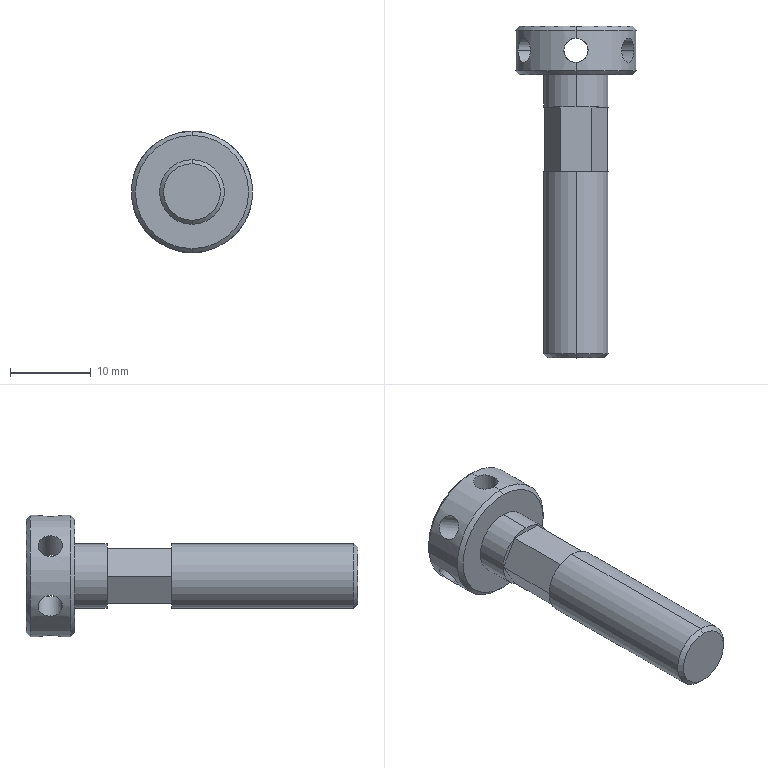Part | SolidWorks | features ICE 3, CirPattern 2, Chamfer 1, Extrusion 1 | 1 solid | 35 faces | box 15 x 41 x 15 mm | volume 2454 mm3 | cylinder 18 | plane 11 | cone 6 | commonest cylinder face diameters 3 x12 8 x4 15 x2
STEP:
#1=CARTESIAN_POINT('',(7.114,38.,2.375));
#2=VERTEX_POINT('',#1);
#3=CARTESIAN_POINT('',(5.614,38.,4.973));
#4=VERTEX_POINT('',#3);
#5=CARTESIAN_POINT('',(7.114,38.,2.375));
#6=CARTESIAN_POINT('',(7.114,37.804,2.375));
#7=CARTESIAN_POINT('',(7.101,37.606,2.414));
#8=CARTESIAN_POINT('',(7.051,37.245,2.557));
#9=CARTESIAN_POINT('',(7.012,37.078,2.664));
#10=CARTESIAN_POINT('',(6.934,36.871,2.858));
#11=CARTESIAN_POINT('',(6.905,36.808,2.93));
#12=CARTESIAN_POINT('',(6.839,36.699,3.079));
#13=CARTESIAN_POINT('',(6.803,36.653,3.158));
#14=CARTESIAN_POINT('',(6.685,36.539,3.405));
#15=CARTESIAN_POINT('',(6.595,36.5,3.578));
#16=CARTESIAN_POINT('',(6.446,36.5,3.835));
#17=CARTESIAN_POINT('',(6.396,36.51,3.919));
#18=CARTESIAN_POINT('',(6.293,36.548,4.081));
#19=CARTESIAN_POINT('',(6.24,36.577,4.161));
#20=CARTESIAN_POINT('',(6.086,36.689,4.386));
#21=CARTESIAN_POINT('',(5.986,36.801,4.521));
#22=CARTESIAN_POINT('',(5.814,37.076,4.74));
#23=CARTESIAN_POINT('',(5.741,37.243,4.827));
#24=CARTESIAN_POINT('',(5.641,37.604,4.943));
#25=CARTESIAN_POINT('',(5.614,37.801,4.973));
#26=CARTESIAN_POINT('',(5.614,38.,4.973));
#27=B_SPLINE_CURVE_WITH_KNOTS('',3,(#5,#6,#7,#8,#9,#10,#11,#12,#13,#14,#15,#16,#17,#18,#19,#20,#21,#22,#23,#24,#25,#26),.UNSPECIFIED.,.F.,.F.,(4,2,2,2,2,2,2,2,2,2,4),(0.004702,0.005289,0.005877,0.00617,0.006464,0.007052,0.007345,0.007639,0.008227,0.008814,0.009402),.UNSPECIFIED.);
#28=EDGE_CURVE('',#2,#4,#27,.T.);
#29=ORIENTED_EDGE('',*,*,#28,.F.);
#30=CARTESIAN_POINT('',(3.,38.,0.));
#31=VERTEX_POINT('',#30);
#32=CARTESIAN_POINT('',(8.977,38.,3.451));
#33=DIRECTION('',(-0.866,0.,-0.5));
#34=VECTOR('',#33,1000.);
#35=LINE('',#32,#34);
#36=EDGE_CURVE('',#2,#31,#35,.T.);
#37=ORIENTED_EDGE('',*,*,#36,.T.);
#38=CARTESIAN_POINT('',(0.,36.5,0.));
#39=VERTEX_POINT('',#38);
#40=CARTESIAN_POINT('',(0.,36.5,0.));
#41=CARTESIAN_POINT('',(1.757,36.5,0.));
#42=CARTESIAN_POINT('',(3.,37.121,0.));
#43=CARTESIAN_POINT('',(3.,38.,0.));
#44=(BOUNDED_CURVE()B_SPLINE_CURVE(3,(#40,#41,#42,#43),.UNSPECIFIED.,.F.,.F.)B_SPLINE_CURVE_WITH_KNOTS((4,4),(4.712,6.283),.UNSPECIFIED.)CURVE()GEOMETRIC_REPRESENTATION_ITEM()RATIONAL_B_SPLINE_CURVE((1.,0.8047,0.8047,1.))REPRESENTATION_ITEM(''));
#45=EDGE_CURVE('',#39,#31,#44,.T.);
#46=ORIENTED_EDGE('',*,*,#45,.F.);
#47=CARTESIAN_POINT('',(1.5,38.,2.598));
#48=VERTEX_POINT('',#47);
#49=CARTESIAN_POINT('',(1.5,38.,2.598));
#50=CARTESIAN_POINT('',(1.5,37.121,2.598));
#51=CARTESIAN_POINT('',(0.8787,36.5,1.522));
#52=CARTESIAN_POINT('',(0.,36.5,0.));
#53=(BOUNDED_CURVE()B_SPLINE_CURVE(3,(#49,#50,#51,#52),.UNSPECIFIED.,.F.,.F.)B_SPLINE_CURVE_WITH_KNOTS((4,4),(3.142,4.712),.UNSPECIFIED.)CURVE()GEOMETRIC_REPRESENTATION_ITEM()RATIONAL_B_SPLINE_CURVE((1.,0.8047,0.8047,1.))REPRESENTATION_ITEM(''));
#54=EDGE_CURVE('',#48,#39,#53,.T.);
#55=ORIENTED_EDGE('',*,*,#54,.F.);
#56=CARTESIAN_POINT('',(7.477,38.,6.049));
#57=DIRECTION('',(-0.866,0.,-0.5));
#58=VECTOR('',#57,1000.);
#59=LINE('',#56,#58);
#60=EDGE_CURVE('',#4,#48,#59,.T.);
#61=ORIENTED_EDGE('',*,*,#60,.F.);
#62=EDGE_LOOP('',(#29,#37,#46,#55,#61));
#63=FACE_OUTER_BOUND('',#62,.T.);
#64=CARTESIAN_POINT('',(8.227,38.,4.75));
#65=DIRECTION('',(-0.866,0.,-0.5));
#66=DIRECTION('',(-0.5,0.,0.866));
#67=AXIS2_PLACEMENT_3D('',#64,#65,#66);
#68=CYLINDRICAL_SURFACE('',#67,1.5);
#69=ADVANCED_FACE('',(#63),#68,.F.);
#70=CARTESIAN_POINT('',(5.614,38.,-4.973));
#71=VERTEX_POINT('',#70);
#72=CARTESIAN_POINT('',(7.114,38.,-2.375));
#73=VERTEX_POINT('',#72);
#74=CARTESIAN_POINT('',(5.614,38.,-4.973));
#75=CARTESIAN_POINT('',(5.614,37.804,-4.973));
#76=CARTESIAN_POINT('',(5.641,37.606,-4.943));
#77=CARTESIAN_POINT('',(5.74,37.245,-4.828));
#78=CARTESIAN_POINT('',(5.813,37.078,-4.741));
#79=CARTESIAN_POINT('',(5.942,36.871,-4.576));
#80=CARTESIAN_POINT('',(5.989,36.808,-4.515));
#81=CARTESIAN_POINT('',(6.086,36.699,-4.383));
#82=CARTESIAN_POINT('',(6.137,36.653,-4.313));
#83=CARTESIAN_POINT('',(6.291,36.539,-4.087));
#84=CARTESIAN_POINT('',(6.396,36.5,-3.922));
#85=CARTESIAN_POINT('',(6.544,36.5,-3.665));
#86=CARTESIAN_POINT('',(6.591,36.51,-3.579));
#87=CARTESIAN_POINT('',(6.681,36.548,-3.409));
#88=CARTESIAN_POINT('',(6.724,36.577,-3.324));
#89=CARTESIAN_POINT('',(6.842,36.689,-3.078));
#90=CARTESIAN_POINT('',(6.908,36.801,-2.924));
#91=CARTESIAN_POINT('',(7.012,37.076,-2.665));
#92=CARTESIAN_POINT('',(7.051,37.243,-2.558));
#93=CARTESIAN_POINT('',(7.101,37.604,-2.414));
#94=CARTESIAN_POINT('',(7.114,37.801,-2.375));
#95=CARTESIAN_POINT('',(7.114,38.,-2.375));
#96=B_SPLINE_CURVE_WITH_KNOTS('',3,(#74,#75,#76,#77,#78,#79,#80,#81,#82,#83,#84,#85,#86,#87,#88,#89,#90,#91,#92,#93,#94,#95),.UNSPECIFIED.,.F.,.F.,(4,2,2,2,2,2,2,2,2,2,4),(0.004702,0.005289,0.005877,0.00617,0.006464,0.007052,0.007345,0.007639,0.008227,0.008814,0.009402),.UNSPECIFIED.);
#97=EDGE_CURVE('',#71,#73,#96,.T.);
#98=ORIENTED_EDGE('',*,*,#97,.F.);
#99=CARTESIAN_POINT('',(1.5,38.,-2.598));
#100=VERTEX_POINT('',#99);
#101=CARTESIAN_POINT('',(7.477,38.,-6.049));
#102=DIRECTION('',(-0.866,0.,0.5));
#103=VECTOR('',#102,1000.);
#104=LINE('',#101,#103);
#105=EDGE_CURVE('',#71,#100,#104,.T.);
#106=ORIENTED_EDGE('',*,*,#105,.T.);
#107=CARTESIAN_POINT('',(0.,36.5,0.));
#108=CARTESIAN_POINT('',(0.8787,36.5,-1.522));
#109=CARTESIAN_POINT('',(1.5,37.121,-2.598));
#110=CARTESIAN_POINT('',(1.5,38.,-2.598));
#111=(BOUNDED_CURVE()B_SPLINE_CURVE(3,(#107,#108,#109,#110),.UNSPECIFIED.,.F.,.F.)B_SPLINE_CURVE_WITH_KNOTS((4,4),(4.712,6.283),.UNSPECIFIED.)CURVE()GEOMETRIC_REPRESENTATION_ITEM()RATIONAL_B_SPLINE_CURVE((1.,0.8047,0.8047,1.))REPRESENTATION_ITEM(''));
#112=EDGE_CURVE('',#39,#100,#111,.T.);
#113=ORIENTED_EDGE('',*,*,#112,.F.);
#114=ORIENTED_EDGE('',*,*,#45,.T.);
#115=CARTESIAN_POINT('',(8.977,38.,-3.451));
#116=DIRECTION('',(-0.866,0.,0.5));
#117=VECTOR('',#116,1000.);
#118=LINE('',#115,#117);
#119=EDGE_CURVE('',#73,#31,#118,.T.);
#120=ORIENTED_EDGE('',*,*,#119,.F.);
#121=EDGE_LOOP('',(#98,#106,#113,#114,#120));
#122=FACE_OUTER_BOUND('',#121,.T.);
#123=CARTESIAN_POINT('',(8.227,38.,-4.75));
#124=DIRECTION('',(-0.866,0.,0.5));
#125=DIRECTION('',(0.5,0.,0.866));
#126=AXIS2_PLACEMENT_3D('',#123,#124,#125);
#127=CYLINDRICAL_SURFACE('',#126,1.5);
#128=ADVANCED_FACE('',(#122),#127,.F.);
#129=CARTESIAN_POINT('',(-3.,38.,0.));
#130=VERTEX_POINT('',#129);
#131=CARTESIAN_POINT('',(0.,36.5,0.));
#132=CARTESIAN_POINT('',(-1.757,36.5,0.));
#133=CARTESIAN_POINT('',(-3.,37.121,0.));
#134=CARTESIAN_POINT('',(-3.,38.,0.));
#135=(BOUNDED_CURVE()B_SPLINE_CURVE(3,(#131,#132,#133,#134),.UNSPECIFIED.,.F.,.F.)B_SPLINE_CURVE_WITH_KNOTS((4,4),(1.571,3.142),.UNSPECIFIED.)CURVE()GEOMETRIC_REPRESENTATION_ITEM()RATIONAL_B_SPLINE_CURVE((1.,0.8047,0.8047,1.))REPRESENTATION_ITEM(''));
#136=EDGE_CURVE('',#39,#130,#135,.T.);
#137=ORIENTED_EDGE('',*,*,#136,.T.);
#138=CARTESIAN_POINT('',(-7.114,38.,2.375));
#139=VERTEX_POINT('',#138);
#140=CARTESIAN_POINT('',(7.477,38.,-6.049));
#141=DIRECTION('',(-0.866,0.,0.5));
#142=VECTOR('',#141,1000.);
#143=LINE('',#140,#142);
#144=EDGE_CURVE('',#130,#139,#143,.T.);
#145=ORIENTED_EDGE('',*,*,#144,.T.);
#146=CARTESIAN_POINT('',(-5.614,38.,4.973));
#147=VERTEX_POINT('',#146);
#148=CARTESIAN_POINT('',(-5.614,38.,4.973));
#149=CARTESIAN_POINT('',(-5.614,37.901,4.973));
#150=CARTESIAN_POINT('',(-5.621,37.803,4.966));
#151=CARTESIAN_POINT('',(-5.646,37.611,4.937));
#152=CARTESIAN_POINT('',(-5.666,37.515,4.914));
#153=CARTESIAN_POINT('',(-5.716,37.334,4.856));
#154=CARTESIAN_POINT('',(-5.746,37.248,4.82));
#155=CARTESIAN_POINT('',(-5.816,37.085,4.735));
#156=CARTESIAN_POINT('',(-5.857,37.008,4.686));
#157=CARTESIAN_POINT('',(-5.986,36.801,4.521));
#158=CARTESIAN_POINT('',(-6.086,36.689,4.386));
#159=CARTESIAN_POINT('',(-6.291,36.54,4.088));
#160=CARTESIAN_POINT('',(-6.397,36.5,3.92));
#161=CARTESIAN_POINT('',(-6.544,36.5,3.666));
#162=CARTESIAN_POINT('',(-6.592,36.51,3.578));
#163=CARTESIAN_POINT('',(-6.682,36.548,3.408));
#164=CARTESIAN_POINT('',(-6.724,36.577,3.324));
#165=CARTESIAN_POINT('',(-6.842,36.69,3.077));
#166=CARTESIAN_POINT('',(-6.908,36.8,2.924));
#167=CARTESIAN_POINT('',(-6.987,37.009,2.728));
#168=CARTESIAN_POINT('',(-7.009,37.085,2.67));
#169=CARTESIAN_POINT('',(-7.047,37.247,2.567));
#170=CARTESIAN_POINT('',(-7.064,37.335,2.522));
#171=CARTESIAN_POINT('',(-7.089,37.516,2.449));
#172=CARTESIAN_POINT('',(-7.098,37.61,2.422));
#173=CARTESIAN_POINT('',(-7.111,37.802,2.385));
#174=CARTESIAN_POINT('',(-7.114,37.902,2.375));
#175=CARTESIAN_POINT('',(-7.114,38.,2.375));
#176=B_SPLINE_CURVE_WITH_KNOTS('',3,(#148,#149,#150,#151,#152,#153,#154,#155,#156,#157,#158,#159,#160,#161,#162,#163,#164,#165,#166,#167,#168,#169,#170,#171,#172,#173,#174,#175),.UNSPECIFIED.,.F.,.F.,(4,2,2,2,2,2,2,2,2,2,2,2,2,4),(0.,0.0002938,0.0005877,0.0008815,0.001175,0.001763,0.002351,0.002645,0.002938,0.003526,0.00382,0.004114,0.004408,0.004702),.UNSPECIFIED.);
#177=EDGE_CURVE('',#147,#139,#176,.T.);
#178=ORIENTED_EDGE('',*,*,#177,.F.);
#179=CARTESIAN_POINT('',(-1.5,38.,2.598));
#180=VERTEX_POINT('',#179);
#181=CARTESIAN_POINT('',(8.977,38.,-3.451));
#182=DIRECTION('',(-0.866,0.,0.5));
#183=VECTOR('',#182,1000.);
#184=LINE('',#181,#183);
#185=EDGE_CURVE('',#180,#147,#184,.T.);
#186=ORIENTED_EDGE('',*,*,#185,.F.);
#187=CARTESIAN_POINT('',(0.,36.5,0.));
#188=CARTESIAN_POINT('',(-0.8787,36.5,1.522));
#189=CARTESIAN_POINT('',(-1.5,37.121,2.598));
#190=CARTESIAN_POINT('',(-1.5,38.,2.598));
#191=(BOUNDED_CURVE()B_SPLINE_CURVE(3,(#187,#188,#189,#190),.UNSPECIFIED.,.F.,.T.)B_SPLINE_CURVE_WITH_KNOTS((4,4),(1.571,3.142),.UNSPECIFIED.)CURVE()GEOMETRIC_REPRESENTATION_ITEM()RATIONAL_B_SPLINE_CURVE((1.,0.8047,0.8047,1.))REPRESENTATION_ITEM(''));
#192=EDGE_CURVE('',#39,#180,#191,.T.);
#193=ORIENTED_EDGE('',*,*,#192,.F.);
#194=EDGE_LOOP('',(#137,#145,#178,#186,#193));
#195=FACE_OUTER_BOUND('',#194,.T.);
#196=CARTESIAN_POINT('',(8.227,38.,-4.75));
#197=DIRECTION('',(-0.866,0.,0.5));
#198=DIRECTION('',(0.5,0.,0.866));
#199=AXIS2_PLACEMENT_3D('',#196,#197,#198);
#200=CYLINDRICAL_SURFACE('',#199,1.5);
#201=ADVANCED_FACE('',(#195),#200,.F.);
#202=CARTESIAN_POINT('',(-1.5,38.,-2.598));
#203=VERTEX_POINT('',#202);
#204=CARTESIAN_POINT('',(-1.5,38.,-2.598));
#205=CARTESIAN_POINT('',(-1.5,37.121,-2.598));
#206=CARTESIAN_POINT('',(-0.8787,36.5,-1.522));
#207=CARTESIAN_POINT('',(0.,36.5,0.));
#208=(BOUNDED_CURVE()B_SPLINE_CURVE(3,(#204,#205,#206,#207),.UNSPECIFIED.,.F.,.F.)B_SPLINE_CURVE_WITH_KNOTS((4,4),(0.,1.571),.UNSPECIFIED.)CURVE()GEOMETRIC_REPRESENTATION_ITEM()RATIONAL_B_SPLINE_CURVE((1.,0.8047,0.8047,1.))REPRESENTATION_ITEM(''));
#209=EDGE_CURVE('',#203,#39,#208,.T.);
#210=ORIENTED_EDGE('',*,*,#209,.F.);
#211=CARTESIAN_POINT('',(-5.614,38.,-4.973));
#212=VERTEX_POINT('',#211);
#213=CARTESIAN_POINT('',(8.977,38.,3.451));
#214=DIRECTION('',(-0.866,0.,-0.5));
#215=VECTOR('',#214,1000.);
#216=LINE('',#213,#215);
#217=EDGE_CURVE('',#203,#212,#216,.T.);
#218=ORIENTED_EDGE('',*,*,#217,.T.);
#219=CARTESIAN_POINT('',(-7.114,38.,-2.375));
#220=VERTEX_POINT('',#219);
#221=CARTESIAN_POINT('',(-7.114,38.,-2.375));
#222=CARTESIAN_POINT('',(-7.114,37.901,-2.375));
#223=CARTESIAN_POINT('',(-7.111,37.803,-2.385));
#224=CARTESIAN_POINT('',(-7.098,37.611,-2.422));
#225=CARTESIAN_POINT('',(-7.089,37.515,-2.45));
#226=CARTESIAN_POINT('',(-7.063,37.334,-2.522));
#227=CARTESIAN_POINT('',(-7.048,37.248,-2.566));
#228=CARTESIAN_POINT('',(-7.009,37.085,-2.67));
#229=CARTESIAN_POINT('',(-6.986,37.008,-2.729));
#230=CARTESIAN_POINT('',(-6.908,36.801,-2.923));
#231=CARTESIAN_POINT('',(-6.842,36.689,-3.078));
#232=CARTESIAN_POINT('',(-6.685,36.54,-3.404));
#233=CARTESIAN_POINT('',(-6.594,36.5,-3.58));
#234=CARTESIAN_POINT('',(-6.446,36.5,-3.834));
#235=CARTESIAN_POINT('',(-6.395,36.51,-3.92));
#236=CARTESIAN_POINT('',(-6.292,36.548,-4.083));
#237=CARTESIAN_POINT('',(-6.24,36.577,-4.161));
#238=CARTESIAN_POINT('',(-6.086,36.69,-4.387));
#239=CARTESIAN_POINT('',(-5.986,36.8,-4.52));
#240=CARTESIAN_POINT('',(-5.856,37.009,-4.686));
#241=CARTESIAN_POINT('',(-5.817,37.085,-4.735));
#242=CARTESIAN_POINT('',(-5.746,37.247,-4.82));
#243=CARTESIAN_POINT('',(-5.716,37.335,-4.856));
#244=CARTESIAN_POINT('',(-5.666,37.516,-4.914));
#245=CARTESIAN_POINT('',(-5.647,37.61,-4.936));
#246=CARTESIAN_POINT('',(-5.621,37.802,-4.966));
#247=CARTESIAN_POINT('',(-5.614,37.902,-4.973));
#248=CARTESIAN_POINT('',(-5.614,38.,-4.973));
#249=B_SPLINE_CURVE_WITH_KNOTS('',3,(#221,#222,#223,#224,#225,#226,#227,#228,#229,#230,#231,#232,#233,#234,#235,#236,#237,#238,#239,#240,#241,#242,#243,#244,#245,#246,#247,#248),.UNSPECIFIED.,.F.,.F.,(4,2,2,2,2,2,2,2,2,2,2,2,2,4),(0.,0.0002938,0.0005877,0.0008815,0.001175,0.001763,0.002351,0.002645,0.002938,0.003526,0.00382,0.004114,0.004408,0.004702),.UNSPECIFIED.);
#250=EDGE_CURVE('',#220,#212,#249,.T.);
#251=ORIENTED_EDGE('',*,*,#250,.F.);
#252=CARTESIAN_POINT('',(7.477,38.,6.049));
#253=DIRECTION('',(-0.866,0.,-0.5));
#254=VECTOR('',#253,1000.);
#255=LINE('',#252,#254);
#256=EDGE_CURVE('',#130,#220,#255,.T.);
#257=ORIENTED_EDGE('',*,*,#256,.F.);
#258=ORIENTED_EDGE('',*,*,#136,.F.);
#259=EDGE_LOOP('',(#210,#218,#251,#257,#258));
#260=FACE_OUTER_BOUND('',#259,.T.);
#261=CARTESIAN_POINT('',(8.227,38.,4.75));
#262=DIRECTION('',(-0.866,0.,-0.5));
#263=DIRECTION('',(-0.5,0.,0.866));
#264=AXIS2_PLACEMENT_3D('',#261,#262,#263);
#265=CYLINDRICAL_SURFACE('',#264,1.5);
#266=ADVANCED_FACE('',(#260),#265,.F.);
#267=ORIENTED_EDGE('',*,*,#192,.T.);
#268=CARTESIAN_POINT('',(-1.5,38.,7.348));
#269=VERTEX_POINT('',#268);
#270=CARTESIAN_POINT('',(-1.5,38.,-9.5));
#271=DIRECTION('',(0.,0.,1.));
#272=VECTOR('',#271,1000.);
#273=LINE('',#270,#272);
#274=EDGE_CURVE('',#180,#269,#273,.T.);
#275=ORIENTED_EDGE('',*,*,#274,.T.);
#276=CARTESIAN_POINT('',(0.,36.5,7.5));
#277=VERTEX_POINT('',#276);
#278=CARTESIAN_POINT('',(0.,36.5,7.5));
#279=CARTESIAN_POINT('',(-0.09809,36.5,7.5));
#280=CARTESIAN_POINT('',(-0.1978,36.51,7.498));
#281=CARTESIAN_POINT('',(-0.3903,36.548,7.49));
#282=CARTESIAN_POINT('',(-0.4839,36.577,7.485));
#283=CARTESIAN_POINT('',(-0.7567,36.69,7.464));
#284=CARTESIAN_POINT('',(-0.9216,36.8,7.444));
#285=CARTESIAN_POINT('',(-1.131,37.009,7.415));
#286=CARTESIAN_POINT('',(-1.192,37.085,7.405));
#287=CARTESIAN_POINT('',(-1.301,37.247,7.386));
#288=CARTESIAN_POINT('',(-1.348,37.335,7.378));
#289=CARTESIAN_POINT('',(-1.423,37.516,7.364));
#290=CARTESIAN_POINT('',(-1.452,37.61,7.358));
#291=CARTESIAN_POINT('',(-1.49,37.802,7.35));
#292=CARTESIAN_POINT('',(-1.5,37.902,7.348));
#293=CARTESIAN_POINT('',(-1.5,38.,7.348));
#294=B_SPLINE_CURVE_WITH_KNOTS('',3,(#278,#279,#280,#281,#282,#283,#284,#285,#286,#287,#288,#289,#290,#291,#292,#293),.UNSPECIFIED.,.F.,.F.,(4,2,2,2,2,2,2,4),(0.002351,0.002645,0.002939,0.003526,0.00382,0.004114,0.004408,0.004702),.UNSPECIFIED.);
#295=EDGE_CURVE('',#277,#269,#294,.T.);
#296=ORIENTED_EDGE('',*,*,#295,.F.);
#297=CARTESIAN_POINT('',(1.5,38.,7.348));
#298=VERTEX_POINT('',#297);
#299=CARTESIAN_POINT('',(1.5,38.,7.348));
#300=CARTESIAN_POINT('',(1.5,37.901,7.348));
#301=CARTESIAN_POINT('',(1.49,37.803,7.35));
#302=CARTESIAN_POINT('',(1.452,37.611,7.358));
#303=CARTESIAN_POINT('',(1.423,37.515,7.364));
#304=CARTESIAN_POINT('',(1.348,37.334,7.378));
#305=CARTESIAN_POINT('',(1.301,37.248,7.386));
#306=CARTESIAN_POINT('',(1.192,37.085,7.405));
#307=CARTESIAN_POINT('',(1.129,37.008,7.415));
#308=CARTESIAN_POINT('',(0.9221,36.801,7.444));
#309=CARTESIAN_POINT('',(0.7551,36.689,7.464));
#310=CARTESIAN_POINT('',(0.3941,36.54,7.492));
#311=CARTESIAN_POINT('',(0.1963,36.5,7.5));
#312=CARTESIAN_POINT('',(0.,36.5,7.5));
#313=B_SPLINE_CURVE_WITH_KNOTS('',3,(#299,#300,#301,#302,#303,#304,#305,#306,#307,#308,#309,#310,#311,#312),.UNSPECIFIED.,.F.,.F.,(4,2,2,2,2,2,4),(0.,0.0002939,0.0005878,0.0008818,0.001176,0.001764,0.002351),.UNSPECIFIED.);
#314=EDGE_CURVE('',#298,#277,#313,.T.);
#315=ORIENTED_EDGE('',*,*,#314,.F.);
#316=CARTESIAN_POINT('',(1.5,38.,-9.5));
#317=DIRECTION('',(0.,0.,1.));
#318=VECTOR('',#317,1000.);
#319=LINE('',#316,#318);
#320=EDGE_CURVE('',#48,#298,#319,.T.);
#321=ORIENTED_EDGE('',*,*,#320,.F.);
#322=ORIENTED_EDGE('',*,*,#54,.T.);
#323=EDGE_LOOP('',(#267,#275,#296,#315,#321,#322));
#324=FACE_OUTER_BOUND('',#323,.T.);
#325=CARTESIAN_POINT('',(0.,38.,-9.5));
#326=DIRECTION('',(0.,0.,1.));
#327=DIRECTION('',(1.,0.,0.));
#328=AXIS2_PLACEMENT_3D('',#325,#326,#327);
#329=CYLINDRICAL_SURFACE('',#328,1.5);
#330=ADVANCED_FACE('',(#324),#329,.F.);
#331=CARTESIAN_POINT('',(0.,0.,-3.5));
#332=VERTEX_POINT('',#331);
#333=CARTESIAN_POINT('',(0.,0.,3.5));
#334=VERTEX_POINT('',#333);
#335=CARTESIAN_POINT('',(0.,0.,0.));
#336=DIRECTION('',(0.,-1.,0.));
#337=DIRECTION('',(0.,0.,1.));
#338=AXIS2_PLACEMENT_3D('',#335,#336,#337);
#339=CIRCLE('',#338,3.5);
#340=EDGE_CURVE('',#332,#334,#339,.T.);
#341=ORIENTED_EDGE('',*,*,#340,.F.);
#342=CARTESIAN_POINT('',(0.,0.5,-4.));
#343=VERTEX_POINT('',#342);
#344=CARTESIAN_POINT('',(0.,0.5,-4.));
#345=DIRECTION('',(0.,0.7071,-0.7071));
#346=VECTOR('',#345,1000.);
#347=LINE('',#344,#346);
#348=EDGE_CURVE('',#332,#343,#347,.T.);
#349=ORIENTED_EDGE('',*,*,#348,.T.);
#350=CARTESIAN_POINT('',(0.,0.5,4.));
#351=VERTEX_POINT('',#350);
#352=CARTESIAN_POINT('',(0.,0.5,0.));
#353=DIRECTION('',(0.,1.,0.));
#354=DIRECTION('',(0.,0.,1.));
#355=AXIS2_PLACEMENT_3D('',#352,#353,#354);
#356=CIRCLE('',#355,4.);
#357=EDGE_CURVE('',#351,#343,#356,.T.);
#358=ORIENTED_EDGE('',*,*,#357,.F.);
#359=CARTESIAN_POINT('',(0.,0.5,4.));
#360=DIRECTION('',(0.,0.7071,0.7071));
#361=VECTOR('',#360,1000.);
#362=LINE('',#359,#361);
#363=EDGE_CURVE('',#334,#351,#362,.T.);
#364=ORIENTED_EDGE('',*,*,#363,.F.);
#365=EDGE_LOOP('',(#341,#349,#358,#364));
#366=FACE_OUTER_BOUND('',#365,.T.);
#367=CARTESIAN_POINT('',(0.,0.5,0.));
#368=DIRECTION('',(0.,1.,0.));
#369=DIRECTION('',(0.,0.,1.));
#370=AXIS2_PLACEMENT_3D('',#367,#368,#369);
#371=CONICAL_SURFACE('',#370,4.,0.7854);
#372=ADVANCED_FACE('',(#366),#371,.T.);
#373=CARTESIAN_POINT('',(0.,41.,7.));
#374=VERTEX_POINT('',#373);
#375=CARTESIAN_POINT('',(0.,41.,-7.));
#376=VERTEX_POINT('',#375);
#377=CARTESIAN_POINT('',(0.,41.,0.));
#378=DIRECTION('',(0.,1.,0.));
#379=DIRECTION('',(0.,0.,1.));
#380=AXIS2_PLACEMENT_3D('',#377,#378,#379);
#381=CIRCLE('',#380,7.);
#382=EDGE_CURVE('',#374,#376,#381,.T.);
#383=ORIENTED_EDGE('',*,*,#382,.F.);
#384=CARTESIAN_POINT('',(0.,40.5,7.5));
#385=VERTEX_POINT('',#384);
#386=CARTESIAN_POINT('',(0.,41.,7.));
#387=DIRECTION('',(0.,-0.7071,0.7071));
#388=VECTOR('',#387,1000.);
#389=LINE('',#386,#388);
#390=EDGE_CURVE('',#374,#385,#389,.T.);
#391=ORIENTED_EDGE('',*,*,#390,.T.);
#392=CARTESIAN_POINT('',(0.,40.5,-7.5));
#393=VERTEX_POINT('',#392);
#394=CARTESIAN_POINT('',(0.,40.5,0.));
#395=DIRECTION('',(0.,-1.,0.));
#396=DIRECTION('',(0.,0.,1.));
#397=AXIS2_PLACEMENT_3D('',#394,#395,#396);
#398=CIRCLE('',#397,7.5);
#399=EDGE_CURVE('',#393,#385,#398,.T.);
#400=ORIENTED_EDGE('',*,*,#399,.F.);
#401=CARTESIAN_POINT('',(0.,41.,-7.));
#402=DIRECTION('',(0.,-0.7071,-0.7071));
#403=VECTOR('',#402,1000.);
#404=LINE('',#401,#403);
#405=EDGE_CURVE('',#376,#393,#404,.T.);
#406=ORIENTED_EDGE('',*,*,#405,.F.);
#407=EDGE_LOOP('',(#383,#391,#400,#406));
#408=FACE_OUTER_BOUND('',#407,.T.);
#409=CARTESIAN_POINT('',(0.,41.,0.));
#410=DIRECTION('',(0.,-1.,0.));
#411=DIRECTION('',(0.,0.,-1.));
#412=AXIS2_PLACEMENT_3D('',#409,#410,#411);
#413=CONICAL_SURFACE('',#412,7.,0.7854);
#414=ADVANCED_FACE('',(#408),#413,.T.);
#415=CARTESIAN_POINT('',(0.,35.,-7.));
#416=VERTEX_POINT('',#415);
#417=CARTESIAN_POINT('',(0.,35.,7.));
#418=VERTEX_POINT('',#417);
#419=CARTESIAN_POINT('',(0.,35.,0.));
#420=DIRECTION('',(0.,-1.,0.));
#421=DIRECTION('',(0.,0.,1.));
#422=AXIS2_PLACEMENT_3D('',#419,#420,#421);
#423=CIRCLE('',#422,7.);
#424=EDGE_CURVE('',#416,#418,#423,.T.);
#425=ORIENTED_EDGE('',*,*,#424,.F.);
#426=CARTESIAN_POINT('',(0.,35.5,-7.5));
#427=VERTEX_POINT('',#426);
#428=CARTESIAN_POINT('',(0.,35.5,-7.5));
#429=DIRECTION('',(0.,0.7071,-0.7071));
#430=VECTOR('',#429,1000.);
#431=LINE('',#428,#430);
#432=EDGE_CURVE('',#416,#427,#431,.T.);
#433=ORIENTED_EDGE('',*,*,#432,.T.);
#434=CARTESIAN_POINT('',(0.,35.5,7.5));
#435=VERTEX_POINT('',#434);
#436=CARTESIAN_POINT('',(0.,35.5,0.));
#437=DIRECTION('',(0.,1.,0.));
#438=DIRECTION('',(0.,0.,1.));
#439=AXIS2_PLACEMENT_3D('',#436,#437,#438);
#440=CIRCLE('',#439,7.5);
#441=EDGE_CURVE('',#435,#427,#440,.T.);
#442=ORIENTED_EDGE('',*,*,#441,.F.);
#443=CARTESIAN_POINT('',(0.,35.5,7.5));
#444=DIRECTION('',(0.,0.7071,0.7071));
#445=VECTOR('',#444,1000.);
#446=LINE('',#443,#445);
#447=EDGE_CURVE('',#418,#435,#446,.T.);
#448=ORIENTED_EDGE('',*,*,#447,.F.);
#449=EDGE_LOOP('',(#425,#433,#442,#448));
#450=FACE_OUTER_BOUND('',#449,.T.);
#451=CARTESIAN_POINT('',(0.,35.5,0.));
#452=DIRECTION('',(0.,1.,0.));
#453=DIRECTION('',(0.,0.,1.));
#454=AXIS2_PLACEMENT_3D('',#451,#452,#453);
#455=CONICAL_SURFACE('',#454,7.5,0.7854);
#456=ADVANCED_FACE('',(#450),#455,.T.);
#457=CARTESIAN_POINT('',(5.614,38.,4.973));
#458=CARTESIAN_POINT('',(5.614,38.099,4.973));
#459=CARTESIAN_POINT('',(5.621,38.197,4.966));
#460=CARTESIAN_POINT('',(5.646,38.389,4.937));
#461=CARTESIAN_POINT('',(5.666,38.485,4.914));
#462=CARTESIAN_POINT('',(5.716,38.666,4.856));
#463=CARTESIAN_POINT('',(5.746,38.752,4.82));
#464=CARTESIAN_POINT('',(5.816,38.915,4.735));
#465=CARTESIAN_POINT('',(5.857,38.992,4.686));
#466=CARTESIAN_POINT('',(5.986,39.199,4.521));
#467=CARTESIAN_POINT('',(6.086,39.311,4.386));
#468=CARTESIAN_POINT('',(6.291,39.46,4.088));
#469=CARTESIAN_POINT('',(6.397,39.5,3.92));
#470=CARTESIAN_POINT('',(6.544,39.5,3.666));
#471=CARTESIAN_POINT('',(6.592,39.49,3.578));
#472=CARTESIAN_POINT('',(6.682,39.452,3.408));
#473=CARTESIAN_POINT('',(6.724,39.423,3.324));
#474=CARTESIAN_POINT('',(6.842,39.31,3.077));
#475=CARTESIAN_POINT('',(6.908,39.2,2.924));
#476=CARTESIAN_POINT('',(6.987,38.991,2.728));
#477=CARTESIAN_POINT('',(7.009,38.915,2.67));
#478=CARTESIAN_POINT('',(7.047,38.753,2.567));
#479=CARTESIAN_POINT('',(7.064,38.665,2.522));
#480=CARTESIAN_POINT('',(7.089,38.484,2.449));
#481=CARTESIAN_POINT('',(7.098,38.39,2.422));
#482=CARTESIAN_POINT('',(7.111,38.198,2.385));
#483=CARTESIAN_POINT('',(7.114,38.098,2.375));
#484=CARTESIAN_POINT('',(7.114,38.,2.375));
#485=B_SPLINE_CURVE_WITH_KNOTS('',3,(#457,#458,#459,#460,#461,#462,#463,#464,#465,#466,#467,#468,#469,#470,#471,#472,#473,#474,#475,#476,#477,#478,#479,#480,#481,#482,#483,#484),.UNSPECIFIED.,.F.,.F.,(4,2,2,2,2,2,2,2,2,2,2,2,2,4),(0.,0.0002938,0.0005877,0.0008815,0.001175,0.001763,0.002351,0.002645,0.002938,0.003526,0.00382,0.004114,0.004408,0.004702),.UNSPECIFIED.);
#486=EDGE_CURVE('',#4,#2,#485,.T.);
#487=ORIENTED_EDGE('',*,*,#486,.T.);
#488=ORIENTED_EDGE('',*,*,#28,.T.);
#489=EDGE_LOOP('',(#487,#488));
#490=FACE_BOUND('',#489,.T.);
#491=CARTESIAN_POINT('',(7.114,38.,-2.375));
#492=CARTESIAN_POINT('',(7.114,38.099,-2.375));
#493=CARTESIAN_POINT('',(7.111,38.197,-2.385));
#494=CARTESIAN_POINT('',(7.098,38.389,-2.422));
#495=CARTESIAN_POINT('',(7.089,38.485,-2.45));
#496=CARTESIAN_POINT('',(7.063,38.666,-2.522));
#497=CARTESIAN_POINT('',(7.048,38.752,-2.566));
#498=CARTESIAN_POINT('',(7.009,38.915,-2.67));
#499=CARTESIAN_POINT('',(6.986,38.992,-2.729));
#500=CARTESIAN_POINT('',(6.908,39.199,-2.923));
#501=CARTESIAN_POINT('',(6.842,39.311,-3.078));
#502=CARTESIAN_POINT('',(6.685,39.46,-3.404));
#503=CARTESIAN_POINT('',(6.594,39.5,-3.58));
#504=CARTESIAN_POINT('',(6.446,39.5,-3.834));
#505=CARTESIAN_POINT('',(6.395,39.49,-3.92));
#506=CARTESIAN_POINT('',(6.292,39.452,-4.083));
#507=CARTESIAN_POINT('',(6.24,39.423,-4.161));
#508=CARTESIAN_POINT('',(6.086,39.31,-4.387));
#509=CARTESIAN_POINT('',(5.986,39.2,-4.52));
#510=CARTESIAN_POINT('',(5.856,38.991,-4.686));
#511=CARTESIAN_POINT('',(5.817,38.915,-4.735));
#512=CARTESIAN_POINT('',(5.746,38.753,-4.82));
#513=CARTESIAN_POINT('',(5.716,38.665,-4.856));
#514=CARTESIAN_POINT('',(5.666,38.484,-4.914));
#515=CARTESIAN_POINT('',(5.647,38.39,-4.936));
#516=CARTESIAN_POINT('',(5.621,38.198,-4.966));
#517=CARTESIAN_POINT('',(5.614,38.098,-4.973));
#518=CARTESIAN_POINT('',(5.614,38.,-4.973));
#519=B_SPLINE_CURVE_WITH_KNOTS('',3,(#491,#492,#493,#494,#495,#496,#497,#498,#499,#500,#501,#502,#503,#504,#505,#506,#507,#508,#509,#510,#511,#512,#513,#514,#515,#516,#517,#518),.UNSPECIFIED.,.F.,.F.,(4,2,2,2,2,2,2,2,2,2,2,2,2,4),(0.,0.0002938,0.0005877,0.0008815,0.001175,0.001763,0.002351,0.002645,0.002938,0.003526,0.00382,0.004114,0.004408,0.004702),.UNSPECIFIED.);
#520=EDGE_CURVE('',#73,#71,#519,.T.);
#521=ORIENTED_EDGE('',*,*,#520,.T.);
#522=ORIENTED_EDGE('',*,*,#97,.T.);
#523=EDGE_LOOP('',(#521,#522));
#524=FACE_BOUND('',#523,.T.);
#525=ORIENTED_EDGE('',*,*,#399,.T.);
#526=CARTESIAN_POINT('',(0.,39.5,7.5));
#527=VERTEX_POINT('',#526);
#528=CARTESIAN_POINT('',(0.,41.,7.5));
#529=DIRECTION('',(0.,-1.,0.));
#530=VECTOR('',#529,1000.);
#531=LINE('',#528,#530);
#532=EDGE_CURVE('',#385,#527,#531,.T.);
#533=ORIENTED_EDGE('',*,*,#532,.T.);
#534=CARTESIAN_POINT('',(0.,39.5,7.5));
#535=CARTESIAN_POINT('',(0.09899,39.5,7.5));
#536=CARTESIAN_POINT('',(0.1965,39.49,7.498));
#537=CARTESIAN_POINT('',(0.3887,39.452,7.491));
#538=CARTESIAN_POINT('',(0.4843,39.423,7.485));
#539=CARTESIAN_POINT('',(0.7559,39.31,7.464));
#540=CARTESIAN_POINT('',(0.9224,39.199,7.444));
#541=CARTESIAN_POINT('',(1.198,38.923,7.405));
#542=CARTESIAN_POINT('',(1.31,38.756,7.385));
#543=CARTESIAN_POINT('',(1.46,38.396,7.357));
#544=CARTESIAN_POINT('',(1.5,38.199,7.348));
#545=CARTESIAN_POINT('',(1.5,38.,7.348));
#546=B_SPLINE_CURVE_WITH_KNOTS('',3,(#534,#535,#536,#537,#538,#539,#540,#541,#542,#543,#544,#545),.UNSPECIFIED.,.F.,.F.,(4,2,2,2,2,4),(0.007052,0.007346,0.00764,0.008227,0.008815,0.009402),.UNSPECIFIED.);
#547=EDGE_CURVE('',#527,#298,#546,.T.);
#548=ORIENTED_EDGE('',*,*,#547,.T.);
#549=ORIENTED_EDGE('',*,*,#314,.T.);
#550=CARTESIAN_POINT('',(0.,41.,7.5));
#551=DIRECTION('',(0.,-1.,0.));
#552=VECTOR('',#551,1000.);
#553=LINE('',#550,#552);
#554=EDGE_CURVE('',#277,#435,#553,.T.);
#555=ORIENTED_EDGE('',*,*,#554,.T.);
#556=ORIENTED_EDGE('',*,*,#441,.T.);
#557=CARTESIAN_POINT('',(0.,36.5,-7.5));
#558=VERTEX_POINT('',#557);
#559=CARTESIAN_POINT('',(0.,41.,-7.5));
#560=DIRECTION('',(0.,-1.,0.));
#561=VECTOR('',#560,1000.);
#562=LINE('',#559,#561);
#563=EDGE_CURVE('',#558,#427,#562,.T.);
#564=ORIENTED_EDGE('',*,*,#563,.F.);
#565=CARTESIAN_POINT('',(1.5,38.,-7.348));
#566=VERTEX_POINT('',#565);
#567=CARTESIAN_POINT('',(0.,36.5,-7.5));
#568=CARTESIAN_POINT('',(0.1961,36.5,-7.5));
#569=CARTESIAN_POINT('',(0.394,36.54,-7.492));
#570=CARTESIAN_POINT('',(0.7552,36.689,-7.464));
#571=CARTESIAN_POINT('',(0.922,36.801,-7.444));
#572=CARTESIAN_POINT('',(1.129,37.008,-7.415));
#573=CARTESIAN_POINT('',(1.193,37.085,-7.405));
#574=CARTESIAN_POINT('',(1.301,37.248,-7.386));
#575=CARTESIAN_POINT('',(1.347,37.334,-7.378));
#576=CARTESIAN_POINT('',(1.461,37.607,-7.357));
#577=CARTESIAN_POINT('',(1.5,37.802,-7.348));
#578=CARTESIAN_POINT('',(1.5,38.,-7.348));
#579=B_SPLINE_CURVE_WITH_KNOTS('',3,(#567,#568,#569,#570,#571,#572,#573,#574,#575,#576,#577,#578),.UNSPECIFIED.,.F.,.F.,(4,2,2,2,2,4),(0.004702,0.005289,0.005877,0.006171,0.006465,0.007052),.UNSPECIFIED.);
#580=EDGE_CURVE('',#558,#566,#579,.T.);
#581=ORIENTED_EDGE('',*,*,#580,.T.);
#582=CARTESIAN_POINT('',(0.,39.5,-7.5));
#583=VERTEX_POINT('',#582);
#584=CARTESIAN_POINT('',(1.5,38.,-7.348));
#585=CARTESIAN_POINT('',(1.5,38.099,-7.348));
#586=CARTESIAN_POINT('',(1.49,38.197,-7.35));
#587=CARTESIAN_POINT('',(1.452,38.389,-7.358));
#588=CARTESIAN_POINT('',(1.423,38.484,-7.364));
#589=CARTESIAN_POINT('',(1.31,38.756,-7.385));
#590=CARTESIAN_POINT('',(1.199,38.922,-7.405));
#591=CARTESIAN_POINT('',(0.9233,39.198,-7.444));
#592=CARTESIAN_POINT('',(0.7565,39.31,-7.464));
#593=CARTESIAN_POINT('',(0.3958,39.46,-7.492));
#594=CARTESIAN_POINT('',(0.1986,39.5,-7.5));
#595=CARTESIAN_POINT('',(0.,39.5,-7.5));
#596=B_SPLINE_CURVE_WITH_KNOTS('',3,(#584,#585,#586,#587,#588,#589,#590,#591,#592,#593,#594,#595),.UNSPECIFIED.,.F.,.F.,(4,2,2,2,2,4),(0.007052,0.007346,0.00764,0.008227,0.008815,0.009402),.UNSPECIFIED.);
#597=EDGE_CURVE('',#566,#583,#596,.T.);
#598=ORIENTED_EDGE('',*,*,#597,.T.);
#599=CARTESIAN_POINT('',(0.,41.,-7.5));
#600=DIRECTION('',(0.,-1.,0.));
#601=VECTOR('',#600,1000.);
#602=LINE('',#599,#601);
#603=EDGE_CURVE('',#393,#583,#602,.T.);
#604=ORIENTED_EDGE('',*,*,#603,.F.);
#605=EDGE_LOOP('',(#525,#533,#548,#549,#555,#556,#564,#581,#598,#604));
#606=FACE_OUTER_BOUND('',#605,.T.);
#607=CARTESIAN_POINT('',(0.,41.,0.));
#608=DIRECTION('',(0.,-1.,0.));
#609=DIRECTION('',(0.,0.,-1.));
#610=AXIS2_PLACEMENT_3D('',#607,#608,#609);
#611=CYLINDRICAL_SURFACE('',#610,7.5);
#612=ADVANCED_FACE('',(#490,#524,#606),#611,.T.);
#613=CARTESIAN_POINT('',(0.,35.,4.));
#614=VERTEX_POINT('',#613);
#615=CARTESIAN_POINT('',(0.,35.,-4.));
#616=VERTEX_POINT('',#615);
#617=CARTESIAN_POINT('',(0.,35.,0.));
#618=DIRECTION('',(0.,1.,0.));
#619=DIRECTION('',(0.,0.,1.));
#620=AXIS2_PLACEMENT_3D('',#617,#618,#619);
#621=CIRCLE('',#620,4.);
#622=EDGE_CURVE('',#614,#616,#621,.T.);
#623=ORIENTED_EDGE('',*,*,#622,.F.);
#624=CARTESIAN_POINT('',(0.,31.,4.));
#625=VERTEX_POINT('',#624);
#626=CARTESIAN_POINT('',(0.,35.,4.));
#627=DIRECTION('',(0.,-1.,0.));
#628=VECTOR('',#627,1000.);
#629=LINE('',#626,#628);
#630=EDGE_CURVE('',#614,#625,#629,.T.);
#631=ORIENTED_EDGE('',*,*,#630,.T.);
#632=CARTESIAN_POINT('',(0.,31.,-4.));
#633=VERTEX_POINT('',#632);
#634=CARTESIAN_POINT('',(0.,31.,0.));
#635=DIRECTION('',(0.,1.,0.));
#636=DIRECTION('',(0.,0.,1.));
#637=AXIS2_PLACEMENT_3D('',#634,#635,#636);
#638=CIRCLE('',#637,4.);
#639=EDGE_CURVE('',#625,#633,#638,.T.);
#640=ORIENTED_EDGE('',*,*,#639,.T.);
#641=CARTESIAN_POINT('',(0.,35.,-4.));
#642=DIRECTION('',(0.,-1.,0.));
#643=VECTOR('',#642,1000.);
#644=LINE('',#641,#643);
#645=EDGE_CURVE('',#616,#633,#644,.T.);
#646=ORIENTED_EDGE('',*,*,#645,.F.);
#647=EDGE_LOOP('',(#623,#631,#640,#646));
#648=FACE_OUTER_BOUND('',#647,.T.);
#649=CARTESIAN_POINT('',(0.,35.,0.));
#650=DIRECTION('',(0.,-1.,0.));
#651=DIRECTION('',(0.,0.,-1.));
#652=AXIS2_PLACEMENT_3D('',#649,#650,#651);
#653=CYLINDRICAL_SURFACE('',#652,4.);
#654=ADVANCED_FACE('',(#648),#653,.T.);
#655=CARTESIAN_POINT('',(-1.5,38.,-7.348));
#656=VERTEX_POINT('',#655);
#657=CARTESIAN_POINT('',(-1.5,38.,-7.348));
#658=CARTESIAN_POINT('',(-1.5,37.902,-7.348));
#659=CARTESIAN_POINT('',(-1.49,37.802,-7.351));
#660=CARTESIAN_POINT('',(-1.452,37.61,-7.358));
#661=CARTESIAN_POINT('',(-1.423,37.516,-7.364));
#662=CARTESIAN_POINT('',(-1.31,37.243,-7.385));
#663=CARTESIAN_POINT('',(-1.2,37.078,-7.405));
#664=CARTESIAN_POINT('',(-0.9907,36.869,-7.435));
#665=CARTESIAN_POINT('',(-0.9152,36.808,-7.444));
#666=CARTESIAN_POINT('',(-0.7529,36.699,-7.463));
#667=CARTESIAN_POINT('',(-0.6651,36.652,-7.471));
#668=CARTESIAN_POINT('',(-0.4838,36.577,-7.485));
#669=CARTESIAN_POINT('',(-0.3903,36.548,-7.49));
#670=CARTESIAN_POINT('',(-0.1976,36.51,-7.498));
#671=CARTESIAN_POINT('',(-0.09801,36.5,-7.5));
#672=CARTESIAN_POINT('',(0.,36.5,-7.5));
#673=B_SPLINE_CURVE_WITH_KNOTS('',3,(#657,#658,#659,#660,#661,#662,#663,#664,#665,#666,#667,#668,#669,#670,#671,#672),.UNSPECIFIED.,.F.,.F.,(4,2,2,2,2,2,2,4),(0.002351,0.002645,0.002939,0.003526,0.00382,0.004114,0.004408,0.004702),.UNSPECIFIED.);
#674=EDGE_CURVE('',#656,#558,#673,.T.);
#675=ORIENTED_EDGE('',*,*,#674,.F.);
#676=CARTESIAN_POINT('',(-1.5,38.,-9.5));
#677=DIRECTION('',(0.,0.,1.));
#678=VECTOR('',#677,1000.);
#679=LINE('',#676,#678);
#680=EDGE_CURVE('',#656,#203,#679,.T.);
#681=ORIENTED_EDGE('',*,*,#680,.T.);
#682=ORIENTED_EDGE('',*,*,#209,.T.);
#683=ORIENTED_EDGE('',*,*,#112,.T.);
#684=CARTESIAN_POINT('',(1.5,38.,-9.5));
#685=DIRECTION('',(0.,0.,1.));
#686=VECTOR('',#685,1000.);
#687=LINE('',#684,#686);
#688=EDGE_CURVE('',#566,#100,#687,.T.);
#689=ORIENTED_EDGE('',*,*,#688,.F.);
#690=ORIENTED_EDGE('',*,*,#580,.F.);
#691=EDGE_LOOP('',(#675,#681,#682,#683,#689,#690));
#692=FACE_OUTER_BOUND('',#691,.T.);
#693=CARTESIAN_POINT('',(0.,38.,-9.5));
#694=DIRECTION('',(0.,0.,1.));
#695=DIRECTION('',(1.,0.,0.));
#696=AXIS2_PLACEMENT_3D('',#693,#694,#695);
#697=CYLINDRICAL_SURFACE('',#696,1.5);
#698=ADVANCED_FACE('',(#692),#697,.F.);
#699=CARTESIAN_POINT('',(0.,23.,-4.));
#700=VERTEX_POINT('',#699);
#701=CARTESIAN_POINT('',(0.,23.,4.));
#702=VERTEX_POINT('',#701);
#703=CARTESIAN_POINT('',(0.,23.,0.));
#704=DIRECTION('',(0.,-1.,0.));
#705=DIRECTION('',(0.,0.,-1.));
#706=AXIS2_PLACEMENT_3D('',#703,#704,#705);
#707=CIRCLE('',#706,4.);
#708=EDGE_CURVE('',#700,#702,#707,.T.);
#709=ORIENTED_EDGE('',*,*,#708,.T.);
#710=CARTESIAN_POINT('',(0.,35.,4.));
#711=DIRECTION('',(0.,-1.,0.));
#712=VECTOR('',#711,1000.);
#713=LINE('',#710,#712);
#714=EDGE_CURVE('',#702,#351,#713,.T.);
#715=ORIENTED_EDGE('',*,*,#714,.T.);
#716=ORIENTED_EDGE('',*,*,#357,.T.);
#717=CARTESIAN_POINT('',(0.,35.,-4.));
#718=DIRECTION('',(0.,-1.,0.));
#719=VECTOR('',#718,1000.);
#720=LINE('',#717,#719);
#721=EDGE_CURVE('',#700,#343,#720,.T.);
#722=ORIENTED_EDGE('',*,*,#721,.F.);
#723=EDGE_LOOP('',(#709,#715,#716,#722));
#724=FACE_OUTER_BOUND('',#723,.T.);
#725=CARTESIAN_POINT('',(0.,35.,0.));
#726=DIRECTION('',(0.,-1.,0.));
#727=DIRECTION('',(0.,0.,-1.));
#728=AXIS2_PLACEMENT_3D('',#725,#726,#727);
#729=CYLINDRICAL_SURFACE('',#728,4.);
#730=ADVANCED_FACE('',(#724),#729,.T.);
#731=ORIENTED_EDGE('',*,*,#714,.F.);
#732=CARTESIAN_POINT('',(0.,23.,0.));
#733=DIRECTION('',(0.,-1.,0.));
#734=DIRECTION('',(0.,0.,-1.));
#735=AXIS2_PLACEMENT_3D('',#732,#733,#734);
#736=CIRCLE('',#735,4.);
#737=EDGE_CURVE('',#702,#700,#736,.T.);
#738=ORIENTED_EDGE('',*,*,#737,.T.);
#739=ORIENTED_EDGE('',*,*,#721,.T.);
#740=CARTESIAN_POINT('',(0.,0.5,0.));
#741=DIRECTION('',(0.,1.,0.));
#742=DIRECTION('',(0.,0.,1.));
#743=AXIS2_PLACEMENT_3D('',#740,#741,#742);
#744=CIRCLE('',#743,4.);
#745=EDGE_CURVE('',#343,#351,#744,.T.);
#746=ORIENTED_EDGE('',*,*,#745,.T.);
#747=EDGE_LOOP('',(#731,#738,#739,#746));
#748=FACE_OUTER_BOUND('',#747,.T.);
#749=CARTESIAN_POINT('',(0.,35.,0.));
#750=DIRECTION('',(0.,-1.,0.));
#751=DIRECTION('',(0.,0.,-1.));
#752=AXIS2_PLACEMENT_3D('',#749,#750,#751);
#753=CYLINDRICAL_SURFACE('',#752,4.);
#754=ADVANCED_FACE('',(#748),#753,.T.);
#755=ORIENTED_EDGE('',*,*,#680,.F.);
#756=CARTESIAN_POINT('',(0.,39.5,-7.5));
#757=CARTESIAN_POINT('',(-0.0994,39.5,-7.5));
#758=CARTESIAN_POINT('',(-0.1971,39.49,-7.498));
#759=CARTESIAN_POINT('',(-0.3892,39.452,-7.491));
#760=CARTESIAN_POINT('',(-0.4847,39.423,-7.485));
#761=CARTESIAN_POINT('',(-0.6662,39.348,-7.471));
#762=CARTESIAN_POINT('',(-0.7523,39.301,-7.463));
#763=CARTESIAN_POINT('',(-0.9152,39.192,-7.444));
#764=CARTESIAN_POINT('',(-0.9921,39.129,-7.434));
#765=CARTESIAN_POINT('',(-1.199,38.922,-7.405));
#766=CARTESIAN_POINT('',(-1.311,38.755,-7.385));
#767=CARTESIAN_POINT('',(-1.46,38.394,-7.357));
#768=CARTESIAN_POINT('',(-1.5,38.196,-7.348));
#769=CARTESIAN_POINT('',(-1.5,38.,-7.348));
#770=B_SPLINE_CURVE_WITH_KNOTS('',3,(#756,#757,#758,#759,#760,#761,#762,#763,#764,#765,#766,#767,#768,#769),.UNSPECIFIED.,.F.,.F.,(4,2,2,2,2,2,4),(0.,0.0002939,0.0005878,0.0008818,0.001176,0.001764,0.002351),.UNSPECIFIED.);
#771=EDGE_CURVE('',#583,#656,#770,.T.);
#772=ORIENTED_EDGE('',*,*,#771,.F.);
#773=ORIENTED_EDGE('',*,*,#597,.F.);
#774=ORIENTED_EDGE('',*,*,#688,.T.);
#775=CARTESIAN_POINT('',(0.,39.5,0.));
#776=VERTEX_POINT('',#775);
#777=CARTESIAN_POINT('',(1.5,38.,-2.598));
#778=CARTESIAN_POINT('',(1.5,38.879,-2.598));
#779=CARTESIAN_POINT('',(0.8787,39.5,-1.522));
#780=CARTESIAN_POINT('',(0.,39.5,0.));
#781=(BOUNDED_CURVE()B_SPLINE_CURVE(3,(#777,#778,#779,#780),.UNSPECIFIED.,.F.,.T.)B_SPLINE_CURVE_WITH_KNOTS((4,4),(0.,1.571),.UNSPECIFIED.)CURVE()GEOMETRIC_REPRESENTATION_ITEM()RATIONAL_B_SPLINE_CURVE((1.,0.8047,0.8047,1.))REPRESENTATION_ITEM(''));
#782=EDGE_CURVE('',#100,#776,#781,.T.);
#783=ORIENTED_EDGE('',*,*,#782,.T.);
#784=CARTESIAN_POINT('',(0.,39.5,0.));
#785=CARTESIAN_POINT('',(-0.8787,39.5,-1.522));
#786=CARTESIAN_POINT('',(-1.5,38.879,-2.598));
#787=CARTESIAN_POINT('',(-1.5,38.,-2.598));
#788=(BOUNDED_CURVE()B_SPLINE_CURVE(3,(#784,#785,#786,#787),.UNSPECIFIED.,.F.,.F.)B_SPLINE_CURVE_WITH_KNOTS((4,4),(4.712,6.283),.UNSPECIFIED.)CURVE()GEOMETRIC_REPRESENTATION_ITEM()RATIONAL_B_SPLINE_CURVE((1.,0.8047,0.8047,1.))REPRESENTATION_ITEM(''));
#789=EDGE_CURVE('',#776,#203,#788,.T.);
#790=ORIENTED_EDGE('',*,*,#789,.T.);
#791=EDGE_LOOP('',(#755,#772,#773,#774,#783,#790));
#792=FACE_OUTER_BOUND('',#791,.T.);
#793=CARTESIAN_POINT('',(0.,38.,-9.5));
#794=DIRECTION('',(0.,0.,1.));
#795=DIRECTION('',(1.,0.,0.));
#796=AXIS2_PLACEMENT_3D('',#793,#794,#795);
#797=CYLINDRICAL_SURFACE('',#796,1.5);
#798=ADVANCED_FACE('',(#792),#797,.F.);
#799=ORIENTED_EDGE('',*,*,#630,.F.);
#800=CARTESIAN_POINT('',(0.,35.,0.));
#801=DIRECTION('',(0.,1.,0.));
#802=DIRECTION('',(0.,0.,1.));
#803=AXIS2_PLACEMENT_3D('',#800,#801,#802);
#804=CIRCLE('',#803,4.);
#805=EDGE_CURVE('',#616,#614,#804,.T.);
#806=ORIENTED_EDGE('',*,*,#805,.F.);
#807=ORIENTED_EDGE('',*,*,#645,.T.);
#808=CARTESIAN_POINT('',(0.,31.,0.));
#809=DIRECTION('',(0.,1.,0.));
#810=DIRECTION('',(0.,0.,1.));
#811=AXIS2_PLACEMENT_3D('',#808,#809,#810);
#812=CIRCLE('',#811,4.);
#813=EDGE_CURVE('',#633,#625,#812,.T.);
#814=ORIENTED_EDGE('',*,*,#813,.T.);
#815=EDGE_LOOP('',(#799,#806,#807,#814));
#816=FACE_OUTER_BOUND('',#815,.T.);
#817=CARTESIAN_POINT('',(0.,35.,0.));
#818=DIRECTION('',(0.,-1.,0.));
#819=DIRECTION('',(0.,0.,-1.));
#820=AXIS2_PLACEMENT_3D('',#817,#818,#819);
#821=CYLINDRICAL_SURFACE('',#820,4.);
#822=ADVANCED_FACE('',(#816),#821,.T.);
#823=CARTESIAN_POINT('',(0.,0.,0.));
#824=DIRECTION('',(0.,-1.,0.));
#825=DIRECTION('',(0.,0.,1.));
#826=AXIS2_PLACEMENT_3D('',#823,#824,#825);
#827=CIRCLE('',#826,3.5);
#828=EDGE_CURVE('',#334,#332,#827,.T.);
#829=ORIENTED_EDGE('',*,*,#828,.T.);
#830=ORIENTED_EDGE('',*,*,#340,.T.);
#831=EDGE_LOOP('',(#829,#830));
#832=FACE_OUTER_BOUND('',#831,.T.);
#833=CARTESIAN_POINT('',(0.,0.,0.));
#834=DIRECTION('',(0.,1.,0.));
#835=DIRECTION('',(0.,0.,1.));
#836=AXIS2_PLACEMENT_3D('',#833,#834,#835);
#837=PLANE('',#836);
#838=ADVANCED_FACE('',(#832),#837,.F.);
#839=CARTESIAN_POINT('',(0.,35.,0.));
#840=DIRECTION('',(0.,-1.,0.));
#841=DIRECTION('',(0.,0.,1.));
#842=AXIS2_PLACEMENT_3D('',#839,#840,#841);
#843=CIRCLE('',#842,7.);
#844=EDGE_CURVE('',#418,#416,#843,.T.);
#845=ORIENTED_EDGE('',*,*,#844,.T.);
#846=ORIENTED_EDGE('',*,*,#424,.T.);
#847=EDGE_LOOP('',(#845,#846));
#848=FACE_OUTER_BOUND('',#847,.T.);
#849=ORIENTED_EDGE('',*,*,#805,.T.);
#850=ORIENTED_EDGE('',*,*,#622,.T.);
#851=EDGE_LOOP('',(#849,#850));
#852=FACE_BOUND('',#851,.T.);
#853=CARTESIAN_POINT('',(0.,35.,0.));
#854=DIRECTION('',(0.,1.,0.));
#855=DIRECTION('',(0.,0.,1.));
#856=AXIS2_PLACEMENT_3D('',#853,#854,#855);
#857=PLANE('',#856);
#858=ADVANCED_FACE('',(#848,#852),#857,.F.);
#859=ORIENTED_EDGE('',*,*,#532,.F.);
#860=CARTESIAN_POINT('',(0.,40.5,0.));
#861=DIRECTION('',(0.,-1.,0.));
#862=DIRECTION('',(0.,0.,1.));
#863=AXIS2_PLACEMENT_3D('',#860,#861,#862);
#864=CIRCLE('',#863,7.5);
#865=EDGE_CURVE('',#385,#393,#864,.T.);
#866=ORIENTED_EDGE('',*,*,#865,.T.);
#867=ORIENTED_EDGE('',*,*,#603,.T.);
#868=ORIENTED_EDGE('',*,*,#771,.T.);
#869=ORIENTED_EDGE('',*,*,#674,.T.);
#870=ORIENTED_EDGE('',*,*,#563,.T.);
#871=CARTESIAN_POINT('',(0.,35.5,0.));
#872=DIRECTION('',(0.,1.,0.));
#873=DIRECTION('',(0.,0.,1.));
#874=AXIS2_PLACEMENT_3D('',#871,#872,#873);
#875=CIRCLE('',#874,7.5);
#876=EDGE_CURVE('',#427,#435,#875,.T.);
#877=ORIENTED_EDGE('',*,*,#876,.T.);
#878=ORIENTED_EDGE('',*,*,#554,.F.);
#879=ORIENTED_EDGE('',*,*,#295,.T.);
#880=CARTESIAN_POINT('',(-1.5,38.,7.348));
#881=CARTESIAN_POINT('',(-1.5,38.196,7.348));
#882=CARTESIAN_POINT('',(-1.46,38.394,7.357));
#883=CARTESIAN_POINT('',(-1.311,38.755,7.385));
#884=CARTESIAN_POINT('',(-1.199,38.922,7.405));
#885=CARTESIAN_POINT('',(-0.9919,39.129,7.434));
#886=CARTESIAN_POINT('',(-0.9149,39.193,7.444));
#887=CARTESIAN_POINT('',(-0.7525,39.301,7.463));
#888=CARTESIAN_POINT('',(-0.6664,39.347,7.471));
#889=CARTESIAN_POINT('',(-0.3933,39.461,7.492));
#890=CARTESIAN_POINT('',(-0.1981,39.5,7.5));
#891=CARTESIAN_POINT('',(0.,39.5,7.5));
#892=B_SPLINE_CURVE_WITH_KNOTS('',3,(#880,#881,#882,#883,#884,#885,#886,#887,#888,#889,#890,#891),.UNSPECIFIED.,.F.,.F.,(4,2,2,2,2,4),(0.004702,0.005289,0.005877,0.006171,0.006465,0.007052),.UNSPECIFIED.);
#893=EDGE_CURVE('',#269,#527,#892,.T.);
#894=ORIENTED_EDGE('',*,*,#893,.T.);
#895=EDGE_LOOP('',(#859,#866,#867,#868,#869,#870,#877,#878,#879,#894));
#896=FACE_OUTER_BOUND('',#895,.T.);
#897=ORIENTED_EDGE('',*,*,#177,.T.);
#898=CARTESIAN_POINT('',(-7.114,38.,2.375));
#899=CARTESIAN_POINT('',(-7.114,38.196,2.375));
#900=CARTESIAN_POINT('',(-7.101,38.394,2.414));
#901=CARTESIAN_POINT('',(-7.051,38.755,2.557));
#902=CARTESIAN_POINT('',(-7.012,38.922,2.664));
#903=CARTESIAN_POINT('',(-6.934,39.129,2.858));
#904=CARTESIAN_POINT('',(-6.905,39.192,2.93));
#905=CARTESIAN_POINT('',(-6.839,39.301,3.079));
#906=CARTESIAN_POINT('',(-6.803,39.347,3.158));
#907=CARTESIAN_POINT('',(-6.685,39.461,3.405));
#908=CARTESIAN_POINT('',(-6.595,39.5,3.578));
#909=CARTESIAN_POINT('',(-6.446,39.5,3.835));
#910=CARTESIAN_POINT('',(-6.396,39.49,3.919));
#911=CARTESIAN_POINT('',(-6.293,39.452,4.081));
#912=CARTESIAN_POINT('',(-6.24,39.423,4.161));
#913=CARTESIAN_POINT('',(-6.086,39.311,4.386));
#914=CARTESIAN_POINT('',(-5.986,39.199,4.521));
#915=CARTESIAN_POINT('',(-5.814,38.924,4.74));
#916=CARTESIAN_POINT('',(-5.741,38.757,4.827));
#917=CARTESIAN_POINT('',(-5.641,38.396,4.943));
#918=CARTESIAN_POINT('',(-5.614,38.199,4.973));
#919=CARTESIAN_POINT('',(-5.614,38.,4.973));
#920=B_SPLINE_CURVE_WITH_KNOTS('',3,(#898,#899,#900,#901,#902,#903,#904,#905,#906,#907,#908,#909,#910,#911,#912,#913,#914,#915,#916,#917,#918,#919),.UNSPECIFIED.,.F.,.F.,(4,2,2,2,2,2,2,2,2,2,4),(0.004702,0.005289,0.005877,0.00617,0.006464,0.007052,0.007345,0.007639,0.008227,0.008814,0.009402),.UNSPECIFIED.);
#921=EDGE_CURVE('',#139,#147,#920,.T.);
#922=ORIENTED_EDGE('',*,*,#921,.T.);
#923=EDGE_LOOP('',(#897,#922));
#924=FACE_BOUND('',#923,.T.);
#925=ORIENTED_EDGE('',*,*,#250,.T.);
#926=CARTESIAN_POINT('',(-5.614,38.,-4.973));
#927=CARTESIAN_POINT('',(-5.614,38.196,-4.973));
#928=CARTESIAN_POINT('',(-5.641,38.394,-4.943));
#929=CARTESIAN_POINT('',(-5.74,38.755,-4.828));
#930=CARTESIAN_POINT('',(-5.813,38.922,-4.741));
#931=CARTESIAN_POINT('',(-5.942,39.129,-4.576));
#932=CARTESIAN_POINT('',(-5.989,39.192,-4.515));
#933=CARTESIAN_POINT('',(-6.086,39.301,-4.383));
#934=CARTESIAN_POINT('',(-6.137,39.347,-4.313));
#935=CARTESIAN_POINT('',(-6.291,39.461,-4.087));
#936=CARTESIAN_POINT('',(-6.396,39.5,-3.922));
#937=CARTESIAN_POINT('',(-6.544,39.5,-3.665));
#938=CARTESIAN_POINT('',(-6.591,39.49,-3.579));
#939=CARTESIAN_POINT('',(-6.681,39.452,-3.409));
#940=CARTESIAN_POINT('',(-6.724,39.423,-3.324));
#941=CARTESIAN_POINT('',(-6.842,39.311,-3.078));
#942=CARTESIAN_POINT('',(-6.908,39.199,-2.924));
#943=CARTESIAN_POINT('',(-7.012,38.924,-2.665));
#944=CARTESIAN_POINT('',(-7.051,38.757,-2.558));
#945=CARTESIAN_POINT('',(-7.101,38.396,-2.414));
#946=CARTESIAN_POINT('',(-7.114,38.199,-2.375));
#947=CARTESIAN_POINT('',(-7.114,38.,-2.375));
#948=B_SPLINE_CURVE_WITH_KNOTS('',3,(#926,#927,#928,#929,#930,#931,#932,#933,#934,#935,#936,#937,#938,#939,#940,#941,#942,#943,#944,#945,#946,#947),.UNSPECIFIED.,.F.,.F.,(4,2,2,2,2,2,2,2,2,2,4),(0.004702,0.005289,0.005877,0.00617,0.006464,0.007052,0.007345,0.007639,0.008227,0.008814,0.009402),.UNSPECIFIED.);
#949=EDGE_CURVE('',#212,#220,#948,.T.);
#950=ORIENTED_EDGE('',*,*,#949,.T.);
#951=EDGE_LOOP('',(#925,#950));
#952=FACE_BOUND('',#951,.T.);
#953=CARTESIAN_POINT('',(0.,41.,0.));
#954=DIRECTION('',(0.,-1.,0.));
#955=DIRECTION('',(0.,0.,-1.));
#956=AXIS2_PLACEMENT_3D('',#953,#954,#955);
#957=CYLINDRICAL_SURFACE('',#956,7.5);
#958=ADVANCED_FACE('',(#896,#924,#952),#957,.T.);
#959=CARTESIAN_POINT('',(0.,41.,0.));
#960=DIRECTION('',(0.,1.,0.));
#961=DIRECTION('',(0.,0.,1.));
#962=AXIS2_PLACEMENT_3D('',#959,#960,#961);
#963=CIRCLE('',#962,7.);
#964=EDGE_CURVE('',#376,#374,#963,.T.);
#965=ORIENTED_EDGE('',*,*,#964,.T.);
#966=ORIENTED_EDGE('',*,*,#382,.T.);
#967=EDGE_LOOP('',(#965,#966));
#968=FACE_OUTER_BOUND('',#967,.T.);
#969=CARTESIAN_POINT('',(0.,41.,0.));
#970=DIRECTION('',(0.,1.,0.));
#971=DIRECTION('',(0.,0.,1.));
#972=AXIS2_PLACEMENT_3D('',#969,#970,#971);
#973=PLANE('',#972);
#974=ADVANCED_FACE('',(#968),#973,.T.);
#975=ORIENTED_EDGE('',*,*,#432,.F.);
#976=ORIENTED_EDGE('',*,*,#844,.F.);
#977=ORIENTED_EDGE('',*,*,#447,.T.);
#978=ORIENTED_EDGE('',*,*,#876,.F.);
#979=EDGE_LOOP('',(#975,#976,#977,#978));
#980=FACE_OUTER_BOUND('',#979,.T.);
#981=CARTESIAN_POINT('',(0.,35.5,0.));
#982=DIRECTION('',(0.,1.,0.));
#983=DIRECTION('',(0.,0.,1.));
#984=AXIS2_PLACEMENT_3D('',#981,#982,#983);
#985=CONICAL_SURFACE('',#984,7.5,0.7854);
#986=ADVANCED_FACE('',(#980),#985,.T.);
#987=ORIENTED_EDGE('',*,*,#390,.F.);
#988=ORIENTED_EDGE('',*,*,#964,.F.);
#989=ORIENTED_EDGE('',*,*,#405,.T.);
#990=ORIENTED_EDGE('',*,*,#865,.F.);
#991=EDGE_LOOP('',(#987,#988,#989,#990));
#992=FACE_OUTER_BOUND('',#991,.T.);
#993=CARTESIAN_POINT('',(0.,41.,0.));
#994=DIRECTION('',(0.,-1.,0.));
#995=DIRECTION('',(0.,0.,-1.));
#996=AXIS2_PLACEMENT_3D('',#993,#994,#995);
#997=CONICAL_SURFACE('',#996,7.,0.7854);
#998=ADVANCED_FACE('',(#992),#997,.T.);
#999=ORIENTED_EDGE('',*,*,#348,.F.);
#1000=ORIENTED_EDGE('',*,*,#828,.F.);
#1001=ORIENTED_EDGE('',*,*,#363,.T.);
#1002=ORIENTED_EDGE('',*,*,#745,.F.);
#1003=EDGE_LOOP('',(#999,#1000,#1001,#1002));
#1004=FACE_OUTER_BOUND('',#1003,.T.);
#1005=CARTESIAN_POINT('',(0.,0.5,0.));
#1006=DIRECTION('',(0.,1.,0.));
#1007=DIRECTION('',(0.,0.,1.));
#1008=AXIS2_PLACEMENT_3D('',#1005,#1006,#1007);
#1009=CONICAL_SURFACE('',#1008,4.,0.7854);
#1010=ADVANCED_FACE('',(#1004),#1009,.T.);
#1011=ORIENTED_EDGE('',*,*,#274,.F.);
#1012=CARTESIAN_POINT('',(-1.5,38.,2.598));
#1013=CARTESIAN_POINT('',(-1.5,38.879,2.598));
#1014=CARTESIAN_POINT('',(-0.8787,39.5,1.522));
#1015=CARTESIAN_POINT('',(0.,39.5,0.));
#1016=(BOUNDED_CURVE()B_SPLINE_CURVE(3,(#1012,#1013,#1014,#1015),.UNSPECIFIED.,.F.,.T.)B_SPLINE_CURVE_WITH_KNOTS((4,4),(3.142,4.712),.UNSPECIFIED.)CURVE()GEOMETRIC_REPRESENTATION_ITEM()RATIONAL_B_SPLINE_CURVE((1.,0.8047,0.8047,1.))REPRESENTATION_ITEM(''));
#1017=EDGE_CURVE('',#180,#776,#1016,.T.);
#1018=ORIENTED_EDGE('',*,*,#1017,.T.);
#1019=CARTESIAN_POINT('',(0.,39.5,0.));
#1020=CARTESIAN_POINT('',(0.8787,39.5,1.522));
#1021=CARTESIAN_POINT('',(1.5,38.879,2.598));
#1022=CARTESIAN_POINT('',(1.5,38.,2.598));
#1023=(BOUNDED_CURVE()B_SPLINE_CURVE(3,(#1019,#1020,#1021,#1022),.UNSPECIFIED.,.F.,.F.)B_SPLINE_CURVE_WITH_KNOTS((4,4),(1.571,3.142),.UNSPECIFIED.)CURVE()GEOMETRIC_REPRESENTATION_ITEM()RATIONAL_B_SPLINE_CURVE((1.,0.8047,0.8047,1.))REPRESENTATION_ITEM(''));
#1024=EDGE_CURVE('',#776,#48,#1023,.T.);
#1025=ORIENTED_EDGE('',*,*,#1024,.T.);
#1026=ORIENTED_EDGE('',*,*,#320,.T.);
#1027=ORIENTED_EDGE('',*,*,#547,.F.);
#1028=ORIENTED_EDGE('',*,*,#893,.F.);
#1029=EDGE_LOOP('',(#1011,#1018,#1025,#1026,#1027,#1028));
#1030=FACE_OUTER_BOUND('',#1029,.T.);
#1031=CARTESIAN_POINT('',(0.,38.,-9.5));
#1032=DIRECTION('',(0.,0.,1.));
#1033=DIRECTION('',(1.,0.,0.));
#1034=AXIS2_PLACEMENT_3D('',#1031,#1032,#1033);
#1035=CYLINDRICAL_SURFACE('',#1034,1.5);
#1036=ADVANCED_FACE('',(#1030),#1035,.F.);
#1037=ORIENTED_EDGE('',*,*,#217,.F.);
#1038=ORIENTED_EDGE('',*,*,#789,.F.);
#1039=CARTESIAN_POINT('',(-3.,38.,0.));
#1040=CARTESIAN_POINT('',(-3.,38.879,0.));
#1041=CARTESIAN_POINT('',(-1.757,39.5,0.));
#1042=CARTESIAN_POINT('',(0.,39.5,0.));
#1043=(BOUNDED_CURVE()B_SPLINE_CURVE(3,(#1039,#1040,#1041,#1042),.UNSPECIFIED.,.F.,.T.)B_SPLINE_CURVE_WITH_KNOTS((4,4),(3.142,4.712),.UNSPECIFIED.)CURVE()GEOMETRIC_REPRESENTATION_ITEM()RATIONAL_B_SPLINE_CURVE((1.,0.8047,0.8047,1.))REPRESENTATION_ITEM(''));
#1044=EDGE_CURVE('',#130,#776,#1043,.T.);
#1045=ORIENTED_EDGE('',*,*,#1044,.F.);
#1046=ORIENTED_EDGE('',*,*,#256,.T.);
#1047=ORIENTED_EDGE('',*,*,#949,.F.);
#1048=EDGE_LOOP('',(#1037,#1038,#1045,#1046,#1047));
#1049=FACE_OUTER_BOUND('',#1048,.T.);
#1050=CARTESIAN_POINT('',(8.227,38.,4.75));
#1051=DIRECTION('',(-0.866,0.,-0.5));
#1052=DIRECTION('',(-0.5,0.,0.866));
#1053=AXIS2_PLACEMENT_3D('',#1050,#1051,#1052);
#1054=CYLINDRICAL_SURFACE('',#1053,1.5);
#1055=ADVANCED_FACE('',(#1049),#1054,.F.);
#1056=ORIENTED_EDGE('',*,*,#144,.F.);
#1057=ORIENTED_EDGE('',*,*,#1044,.T.);
#1058=ORIENTED_EDGE('',*,*,#1017,.F.);
#1059=ORIENTED_EDGE('',*,*,#185,.T.);
#1060=ORIENTED_EDGE('',*,*,#921,.F.);
#1061=EDGE_LOOP('',(#1056,#1057,#1058,#1059,#1060));
#1062=FACE_OUTER_BOUND('',#1061,.T.);
#1063=CARTESIAN_POINT('',(8.227,38.,-4.75));
#1064=DIRECTION('',(-0.866,0.,0.5));
#1065=DIRECTION('',(0.5,0.,0.866));
#1066=AXIS2_PLACEMENT_3D('',#1063,#1064,#1065);
#1067=CYLINDRICAL_SURFACE('',#1066,1.5);
#1068=ADVANCED_FACE('',(#1062),#1067,.F.);
#1069=ORIENTED_EDGE('',*,*,#105,.F.);
#1070=ORIENTED_EDGE('',*,*,#520,.F.);
#1071=ORIENTED_EDGE('',*,*,#119,.T.);
#1072=CARTESIAN_POINT('',(3.,38.,0.));
#1073=CARTESIAN_POINT('',(3.,38.879,0.));
#1074=CARTESIAN_POINT('',(1.757,39.5,0.));
#1075=CARTESIAN_POINT('',(0.,39.5,0.));
#1076=(BOUNDED_CURVE()B_SPLINE_CURVE(3,(#1072,#1073,#1074,#1075),.UNSPECIFIED.,.F.,.F.)B_SPLINE_CURVE_WITH_KNOTS((4,4),(0.,1.571),.UNSPECIFIED.)CURVE()GEOMETRIC_REPRESENTATION_ITEM()RATIONAL_B_SPLINE_CURVE((1.,0.8047,0.8047,1.))REPRESENTATION_ITEM(''));
#1077=EDGE_CURVE('',#31,#776,#1076,.T.);
#1078=ORIENTED_EDGE('',*,*,#1077,.T.);
#1079=ORIENTED_EDGE('',*,*,#782,.F.);
#1080=EDGE_LOOP('',(#1069,#1070,#1071,#1078,#1079));
#1081=FACE_OUTER_BOUND('',#1080,.T.);
#1082=CARTESIAN_POINT('',(8.227,38.,-4.75));
#1083=DIRECTION('',(-0.866,0.,0.5));
#1084=DIRECTION('',(0.5,0.,0.866));
#1085=AXIS2_PLACEMENT_3D('',#1082,#1083,#1084);
#1086=CYLINDRICAL_SURFACE('',#1085,1.5);
#1087=ADVANCED_FACE('',(#1081),#1086,.F.);
#1088=ORIENTED_EDGE('',*,*,#36,.F.);
#1089=ORIENTED_EDGE('',*,*,#486,.F.);
#1090=ORIENTED_EDGE('',*,*,#60,.T.);
#1091=ORIENTED_EDGE('',*,*,#1024,.F.);
#1092=ORIENTED_EDGE('',*,*,#1077,.F.);
#1093=EDGE_LOOP('',(#1088,#1089,#1090,#1091,#1092));
#1094=FACE_OUTER_BOUND('',#1093,.T.);
#1095=CARTESIAN_POINT('',(8.227,38.,4.75));
#1096=DIRECTION('',(-0.866,0.,-0.5));
#1097=DIRECTION('',(-0.5,0.,0.866));
#1098=AXIS2_PLACEMENT_3D('',#1095,#1096,#1097);
#1099=CYLINDRICAL_SURFACE('',#1098,1.5);
#1100=ADVANCED_FACE('',(#1094),#1099,.F.);
#1101=ORIENTED_EDGE('',*,*,#708,.F.);
#1102=ORIENTED_EDGE('',*,*,#737,.F.);
#1103=EDGE_LOOP('',(#1101,#1102));
#1104=FACE_OUTER_BOUND('',#1103,.T.);
#1105=CARTESIAN_POINT('',(-1.963,23.,-3.4));
#1106=VERTEX_POINT('',#1105);
#1107=CARTESIAN_POINT('',(1.963,23.,-3.4));
#1108=VERTEX_POINT('',#1107);
#1109=CARTESIAN_POINT('',(-5.,23.,-3.4));
#1110=DIRECTION('',(1.,0.,0.));
#1111=VECTOR('',#1110,1000.);
#1112=LINE('',#1109,#1111);
#1113=EDGE_CURVE('',#1106,#1108,#1112,.T.);
#1114=ORIENTED_EDGE('',*,*,#1113,.T.);
#1115=CARTESIAN_POINT('',(3.926,23.,0.));
#1116=VERTEX_POINT('',#1115);
#1117=CARTESIAN_POINT('',(0.4445,23.,-6.03));
#1118=DIRECTION('',(0.5,0.,0.866));
#1119=VECTOR('',#1118,1000.);
#1120=LINE('',#1117,#1119);
#1121=EDGE_CURVE('',#1108,#1116,#1120,.T.);
#1122=ORIENTED_EDGE('',*,*,#1121,.T.);
#1123=CARTESIAN_POINT('',(1.963,23.,3.4));
#1124=VERTEX_POINT('',#1123);
#1125=CARTESIAN_POINT('',(5.444,23.,-2.63));
#1126=DIRECTION('',(-0.5,0.,0.866));
#1127=VECTOR('',#1126,1000.);
#1128=LINE('',#1125,#1127);
#1129=EDGE_CURVE('',#1116,#1124,#1128,.T.);
#1130=ORIENTED_EDGE('',*,*,#1129,.T.);
#1131=CARTESIAN_POINT('',(-1.963,23.,3.4));
#1132=VERTEX_POINT('',#1131);
#1133=CARTESIAN_POINT('',(5.,23.,3.4));
#1134=DIRECTION('',(-1.,0.,0.));
#1135=VECTOR('',#1134,1000.);
#1136=LINE('',#1133,#1135);
#1137=EDGE_CURVE('',#1124,#1132,#1136,.T.);
#1138=ORIENTED_EDGE('',*,*,#1137,.T.);
#1139=CARTESIAN_POINT('',(-3.926,23.,0.));
#1140=VERTEX_POINT('',#1139);
#1141=CARTESIAN_POINT('',(-0.4445,23.,6.03));
#1142=DIRECTION('',(-0.5,0.,-0.866));
#1143=VECTOR('',#1142,1000.);
#1144=LINE('',#1141,#1143);
#1145=EDGE_CURVE('',#1132,#1140,#1144,.T.);
#1146=ORIENTED_EDGE('',*,*,#1145,.T.);
#1147=CARTESIAN_POINT('',(-5.444,23.,2.63));
#1148=DIRECTION('',(0.5,0.,-0.866));
#1149=VECTOR('',#1148,1000.);
#1150=LINE('',#1147,#1149);
#1151=EDGE_CURVE('',#1140,#1106,#1150,.T.);
#1152=ORIENTED_EDGE('',*,*,#1151,.T.);
#1153=EDGE_LOOP('',(#1114,#1122,#1130,#1138,#1146,#1152));
#1154=FACE_BOUND('',#1153,.T.);
#1155=CARTESIAN_POINT('',(-5.,23.,-3.4));
#1156=DIRECTION('',(0.,-1.,0.));
#1157=DIRECTION('',(0.,0.,-1.));
#1158=AXIS2_PLACEMENT_3D('',#1155,#1156,#1157);
#1159=PLANE('',#1158);
#1160=ADVANCED_FACE('',(#1104,#1154),#1159,.F.);
#1161=CARTESIAN_POINT('',(-1.963,31.,-3.4));
#1162=VERTEX_POINT('',#1161);
#1163=CARTESIAN_POINT('',(1.963,31.,-3.4));
#1164=VERTEX_POINT('',#1163);
#1165=CARTESIAN_POINT('',(-5.,31.,-3.4));
#1166=DIRECTION('',(1.,0.,0.));
#1167=VECTOR('',#1166,1000.);
#1168=LINE('',#1165,#1167);
#1169=EDGE_CURVE('',#1162,#1164,#1168,.T.);
#1170=ORIENTED_EDGE('',*,*,#1169,.T.);
#1171=CARTESIAN_POINT('',(1.963,31.,-3.4));
#1172=DIRECTION('',(0.,-1.,0.));
#1173=VECTOR('',#1172,1000.);
#1174=LINE('',#1171,#1173);
#1175=EDGE_CURVE('',#1164,#1108,#1174,.T.);
#1176=ORIENTED_EDGE('',*,*,#1175,.T.);
#1177=ORIENTED_EDGE('',*,*,#1113,.F.);
#1178=CARTESIAN_POINT('',(-1.963,31.,-3.4));
#1179=DIRECTION('',(0.,1.,0.));
#1180=VECTOR('',#1179,1000.);
#1181=LINE('',#1178,#1180);
#1182=EDGE_CURVE('',#1106,#1162,#1181,.T.);
#1183=ORIENTED_EDGE('',*,*,#1182,.T.);
#1184=EDGE_LOOP('',(#1170,#1176,#1177,#1183));
#1185=FACE_OUTER_BOUND('',#1184,.T.);
#1186=CARTESIAN_POINT('',(-5.,31.,-3.4));
#1187=DIRECTION('',(0.,0.,1.));
#1188=DIRECTION('',(1.,0.,0.));
#1189=AXIS2_PLACEMENT_3D('',#1186,#1187,#1188);
#1190=PLANE('',#1189);
#1191=ADVANCED_FACE('',(#1185),#1190,.F.);
#1192=ORIENTED_EDGE('',*,*,#813,.F.);
#1193=ORIENTED_EDGE('',*,*,#639,.F.);
#1194=EDGE_LOOP('',(#1192,#1193));
#1195=FACE_OUTER_BOUND('',#1194,.T.);
#1196=CARTESIAN_POINT('',(3.926,31.,0.));
#1197=VERTEX_POINT('',#1196);
#1198=CARTESIAN_POINT('',(0.4445,31.,-6.03));
#1199=DIRECTION('',(0.5,0.,0.866));
#1200=VECTOR('',#1199,1000.);
#1201=LINE('',#1198,#1200);
#1202=EDGE_CURVE('',#1164,#1197,#1201,.T.);
#1203=ORIENTED_EDGE('',*,*,#1202,.F.);
#1204=ORIENTED_EDGE('',*,*,#1169,.F.);
#1205=CARTESIAN_POINT('',(-3.926,31.,0.));
#1206=VERTEX_POINT('',#1205);
#1207=CARTESIAN_POINT('',(-5.444,31.,2.63));
#1208=DIRECTION('',(0.5,0.,-0.866));
#1209=VECTOR('',#1208,1000.);
#1210=LINE('',#1207,#1209);
#1211=EDGE_CURVE('',#1206,#1162,#1210,.T.);
#1212=ORIENTED_EDGE('',*,*,#1211,.F.);
#1213=CARTESIAN_POINT('',(-1.963,31.,3.4));
#1214=VERTEX_POINT('',#1213);
#1215=CARTESIAN_POINT('',(-0.4445,31.,6.03));
#1216=DIRECTION('',(-0.5,0.,-0.866));
#1217=VECTOR('',#1216,1000.);
#1218=LINE('',#1215,#1217);
#1219=EDGE_CURVE('',#1214,#1206,#1218,.T.);
#1220=ORIENTED_EDGE('',*,*,#1219,.F.);
#1221=CARTESIAN_POINT('',(1.963,31.,3.4));
#1222=VERTEX_POINT('',#1221);
#1223=CARTESIAN_POINT('',(5.,31.,3.4));
#1224=DIRECTION('',(-1.,0.,0.));
#1225=VECTOR('',#1224,1000.);
#1226=LINE('',#1223,#1225);
#1227=EDGE_CURVE('',#1222,#1214,#1226,.T.);
#1228=ORIENTED_EDGE('',*,*,#1227,.F.);
#1229=CARTESIAN_POINT('',(5.444,31.,-2.63));
#1230=DIRECTION('',(-0.5,0.,0.866));
#1231=VECTOR('',#1230,1000.);
#1232=LINE('',#1229,#1231);
#1233=EDGE_CURVE('',#1197,#1222,#1232,.T.);
#1234=ORIENTED_EDGE('',*,*,#1233,.F.);
#1235=EDGE_LOOP('',(#1203,#1204,#1212,#1220,#1228,#1234));
#1236=FACE_BOUND('',#1235,.T.);
#1237=CARTESIAN_POINT('',(-5.,31.,-3.4));
#1238=DIRECTION('',(0.,1.,0.));
#1239=DIRECTION('',(0.,0.,1.));
#1240=AXIS2_PLACEMENT_3D('',#1237,#1238,#1239);
#1241=PLANE('',#1240);
#1242=ADVANCED_FACE('',(#1195,#1236),#1241,.F.);
#1243=ORIENTED_EDGE('',*,*,#1202,.T.);
#1244=CARTESIAN_POINT('',(3.926,31.,0.));
#1245=DIRECTION('',(0.,-1.,0.));
#1246=VECTOR('',#1245,1000.);
#1247=LINE('',#1244,#1246);
#1248=EDGE_CURVE('',#1197,#1116,#1247,.T.);
#1249=ORIENTED_EDGE('',*,*,#1248,.T.);
#1250=ORIENTED_EDGE('',*,*,#1121,.F.);
#1251=ORIENTED_EDGE('',*,*,#1175,.F.);
#1252=EDGE_LOOP('',(#1243,#1249,#1250,#1251));
#1253=FACE_OUTER_BOUND('',#1252,.T.);
#1254=CARTESIAN_POINT('',(0.4445,31.,-6.03));
#1255=DIRECTION('',(-0.866,0.,0.5));
#1256=DIRECTION('',(0.5,0.,0.866));
#1257=AXIS2_PLACEMENT_3D('',#1254,#1255,#1256);
#1258=PLANE('',#1257);
#1259=ADVANCED_FACE('',(#1253),#1258,.F.);
#1260=ORIENTED_EDGE('',*,*,#1151,.F.);
#1261=CARTESIAN_POINT('',(-3.926,31.,0.));
#1262=DIRECTION('',(0.,-1.,0.));
#1263=VECTOR('',#1262,1000.);
#1264=LINE('',#1261,#1263);
#1265=EDGE_CURVE('',#1206,#1140,#1264,.T.);
#1266=ORIENTED_EDGE('',*,*,#1265,.F.);
#1267=ORIENTED_EDGE('',*,*,#1211,.T.);
#1268=ORIENTED_EDGE('',*,*,#1182,.F.);
#1269=EDGE_LOOP('',(#1260,#1266,#1267,#1268));
#1270=FACE_OUTER_BOUND('',#1269,.T.);
#1271=CARTESIAN_POINT('',(-5.444,31.,2.63));
#1272=DIRECTION('',(0.866,0.,0.5));
#1273=DIRECTION('',(0.5,0.,-0.866));
#1274=AXIS2_PLACEMENT_3D('',#1271,#1272,#1273);
#1275=PLANE('',#1274);
#1276=ADVANCED_FACE('',(#1270),#1275,.F.);
#1277=ORIENTED_EDGE('',*,*,#1219,.T.);
#1278=ORIENTED_EDGE('',*,*,#1265,.T.);
#1279=ORIENTED_EDGE('',*,*,#1145,.F.);
#1280=CARTESIAN_POINT('',(-1.963,31.,3.4));
#1281=DIRECTION('',(0.,-1.,0.));
#1282=VECTOR('',#1281,1000.);
#1283=LINE('',#1280,#1282);
#1284=EDGE_CURVE('',#1214,#1132,#1283,.T.);
#1285=ORIENTED_EDGE('',*,*,#1284,.F.);
#1286=EDGE_LOOP('',(#1277,#1278,#1279,#1285));
#1287=FACE_OUTER_BOUND('',#1286,.T.);
#1288=CARTESIAN_POINT('',(-0.4445,31.,6.03));
#1289=DIRECTION('',(0.866,0.,-0.5));
#1290=DIRECTION('',(-0.5,0.,-0.866));
#1291=AXIS2_PLACEMENT_3D('',#1288,#1289,#1290);
#1292=PLANE('',#1291);
#1293=ADVANCED_FACE('',(#1287),#1292,.F.);
#1294=ORIENTED_EDGE('',*,*,#1227,.T.);
#1295=ORIENTED_EDGE('',*,*,#1284,.T.);
#1296=ORIENTED_EDGE('',*,*,#1137,.F.);
#1297=CARTESIAN_POINT('',(1.963,31.,3.4));
#1298=DIRECTION('',(0.,-1.,0.));
#1299=VECTOR('',#1298,1000.);
#1300=LINE('',#1297,#1299);
#1301=EDGE_CURVE('',#1222,#1124,#1300,.T.);
#1302=ORIENTED_EDGE('',*,*,#1301,.F.);
#1303=EDGE_LOOP('',(#1294,#1295,#1296,#1302));
#1304=FACE_OUTER_BOUND('',#1303,.T.);
#1305=CARTESIAN_POINT('',(5.,31.,3.4));
#1306=DIRECTION('',(0.,0.,-1.));
#1307=DIRECTION('',(-1.,0.,0.));
#1308=AXIS2_PLACEMENT_3D('',#1305,#1306,#1307);
#1309=PLANE('',#1308);
#1310=ADVANCED_FACE('',(#1304),#1309,.F.);
#1311=ORIENTED_EDGE('',*,*,#1233,.T.);
#1312=ORIENTED_EDGE('',*,*,#1301,.T.);
#1313=ORIENTED_EDGE('',*,*,#1129,.F.);
#1314=ORIENTED_EDGE('',*,*,#1248,.F.);
#1315=EDGE_LOOP('',(#1311,#1312,#1313,#1314));
#1316=FACE_OUTER_BOUND('',#1315,.T.);
#1317=CARTESIAN_POINT('',(5.444,31.,-2.63));
#1318=DIRECTION('',(-0.866,0.,-0.5));
#1319=DIRECTION('',(-0.5,0.,0.866));
#1320=AXIS2_PLACEMENT_3D('',#1317,#1318,#1319);
#1321=PLANE('',#1320);
#1322=ADVANCED_FACE('',(#1316),#1321,.F.);
#1323=CLOSED_SHELL('',(#69,#128,#201,#266,#330,#372,#414,#456,#612,#654,#698,#730,#754,#798,#822,#838,#858,#958,#974,#986,#998,#1010,#1036,#1055,#1068,#1087,#1100,#1160,#1191,#1242,#1259,#1276,#1293,#1310,#1322));
#1324=MANIFOLD_SOLID_BREP('',#1323);
#1325=CARTESIAN_POINT('',(0.,0.,0.));
#1326=DIRECTION('',(0.,0.,1.));
#1327=DIRECTION('',(1.,0.,0.));
#1328=AXIS2_PLACEMENT_3D('',#1325,#1326,#1327);
#1329=(LENGTH_UNIT()NAMED_UNIT(*)SI_UNIT(.MILLI.,.METRE.));
#1330=UNCERTAINTY_MEASURE_WITH_UNIT(LENGTH_MEASURE(0.00001),#1329,'','');
#1331=(NAMED_UNIT(*)PLANE_ANGLE_UNIT()SI_UNIT($,.RADIAN.));
#1332=(NAMED_UNIT(*)SI_UNIT($,.STERADIAN.)SOLID_ANGLE_UNIT());
#1333=(GEOMETRIC_REPRESENTATION_CONTEXT(3)GLOBAL_UNCERTAINTY_ASSIGNED_CONTEXT((#1330))GLOBAL_UNIT_ASSIGNED_CONTEXT((#1329,#1331,#1332))REPRESENTATION_CONTEXT('',''));
#1334=ADVANCED_BREP_SHAPE_REPRESENTATION('',(#1324,#1328),#1333);